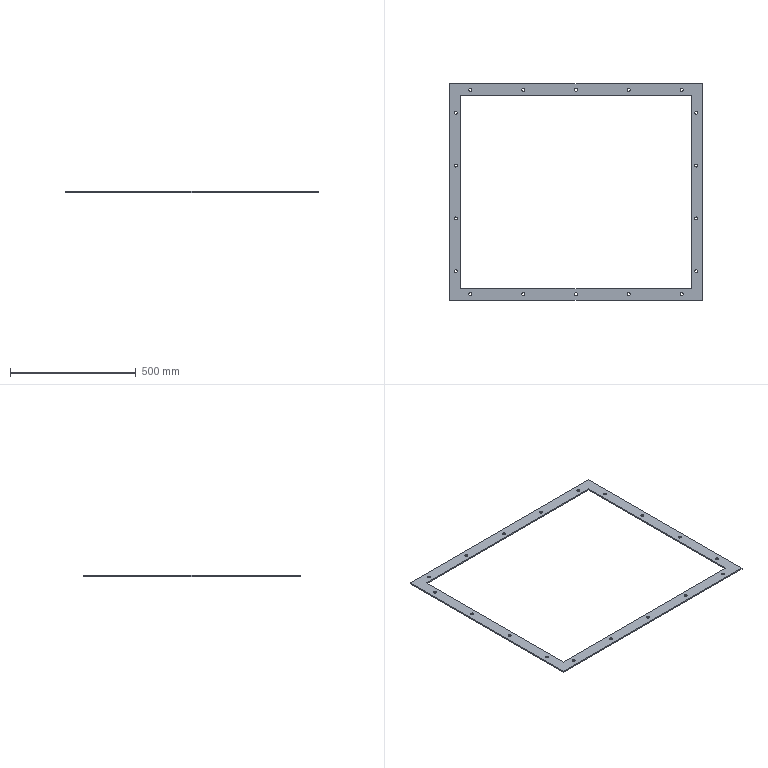Part | STEP file | 750038556 | 1 solid | 46 faces | box 1005 x 861 x 5 mm | volume 789021 mm3 | cylinder 36 | plane 10 | commonest cylinder face diameters 12 x36
STEP:
#1=CARTESIAN_POINT('',(472.,315.,0.));
#2=VERTEX_POINT('',#1);
#3=CARTESIAN_POINT('',(484.,315.,0.));
#4=VERTEX_POINT('',#3);
#5=CARTESIAN_POINT('',(478.,315.,0.));
#6=DIRECTION('',(0.,0.,1.));
#7=DIRECTION('',(1.,0.,0.));
#8=AXIS2_PLACEMENT_3D('',#5,#6,#7);
#9=CIRCLE('',#8,6.);
#10=EDGE_CURVE('',#2,#4,#9,.T.);
#11=ORIENTED_EDGE('',*,*,#10,.F.);
#12=CARTESIAN_POINT('',(472.,315.,5.));
#13=VERTEX_POINT('',#12);
#14=CARTESIAN_POINT('',(472.,315.,-0.5));
#15=DIRECTION('',(0.,0.,1.));
#16=VECTOR('',#15,1000.);
#17=LINE('',#14,#16);
#18=EDGE_CURVE('',#2,#13,#17,.T.);
#19=ORIENTED_EDGE('',*,*,#18,.T.);
#20=CARTESIAN_POINT('',(484.,315.,5.));
#21=VERTEX_POINT('',#20);
#22=CARTESIAN_POINT('',(478.,315.,5.));
#23=DIRECTION('',(0.,0.,-1.));
#24=DIRECTION('',(1.,0.,0.));
#25=AXIS2_PLACEMENT_3D('',#22,#23,#24);
#26=CIRCLE('',#25,6.);
#27=EDGE_CURVE('',#21,#13,#26,.T.);
#28=ORIENTED_EDGE('',*,*,#27,.F.);
#29=CARTESIAN_POINT('',(484.,315.,-0.5));
#30=DIRECTION('',(0.,0.,1.));
#31=VECTOR('',#30,1000.);
#32=LINE('',#29,#31);
#33=EDGE_CURVE('',#4,#21,#32,.T.);
#34=ORIENTED_EDGE('',*,*,#33,.F.);
#35=EDGE_LOOP('',(#11,#19,#28,#34));
#36=FACE_OUTER_BOUND('',#35,.T.);
#37=CARTESIAN_POINT('',(478.,315.,-0.5));
#38=DIRECTION('',(0.,0.,1.));
#39=DIRECTION('',(1.,0.,0.));
#40=AXIS2_PLACEMENT_3D('',#37,#38,#39);
#41=CYLINDRICAL_SURFACE('',#40,6.);
#42=ADVANCED_FACE('',(#36),#41,.F.);
#43=CARTESIAN_POINT('',(-484.,-315.,0.));
#44=VERTEX_POINT('',#43);
#45=CARTESIAN_POINT('',(-472.,-315.,0.));
#46=VERTEX_POINT('',#45);
#47=CARTESIAN_POINT('',(-478.,-315.,0.));
#48=DIRECTION('',(0.,0.,1.));
#49=DIRECTION('',(1.,0.,0.));
#50=AXIS2_PLACEMENT_3D('',#47,#48,#49);
#51=CIRCLE('',#50,6.);
#52=EDGE_CURVE('',#44,#46,#51,.T.);
#53=ORIENTED_EDGE('',*,*,#52,.F.);
#54=CARTESIAN_POINT('',(-484.,-315.,5.));
#55=VERTEX_POINT('',#54);
#56=CARTESIAN_POINT('',(-484.,-315.,-0.5));
#57=DIRECTION('',(0.,0.,1.));
#58=VECTOR('',#57,1000.);
#59=LINE('',#56,#58);
#60=EDGE_CURVE('',#44,#55,#59,.T.);
#61=ORIENTED_EDGE('',*,*,#60,.T.);
#62=CARTESIAN_POINT('',(-472.,-315.,5.));
#63=VERTEX_POINT('',#62);
#64=CARTESIAN_POINT('',(-478.,-315.,5.));
#65=DIRECTION('',(0.,0.,-1.));
#66=DIRECTION('',(1.,0.,0.));
#67=AXIS2_PLACEMENT_3D('',#64,#65,#66);
#68=CIRCLE('',#67,6.);
#69=EDGE_CURVE('',#63,#55,#68,.T.);
#70=ORIENTED_EDGE('',*,*,#69,.F.);
#71=CARTESIAN_POINT('',(-472.,-315.,-0.5));
#72=DIRECTION('',(0.,0.,1.));
#73=VECTOR('',#72,1000.);
#74=LINE('',#71,#73);
#75=EDGE_CURVE('',#46,#63,#74,.T.);
#76=ORIENTED_EDGE('',*,*,#75,.F.);
#77=EDGE_LOOP('',(#53,#61,#70,#76));
#78=FACE_OUTER_BOUND('',#77,.T.);
#79=CARTESIAN_POINT('',(-478.,-315.,-0.5));
#80=DIRECTION('',(0.,0.,1.));
#81=DIRECTION('',(1.,0.,0.));
#82=AXIS2_PLACEMENT_3D('',#79,#80,#81);
#83=CYLINDRICAL_SURFACE('',#82,6.);
#84=ADVANCED_FACE('',(#78),#83,.F.);
#85=CARTESIAN_POINT('',(414.,-406.,0.));
#86=VERTEX_POINT('',#85);
#87=CARTESIAN_POINT('',(426.,-406.,0.));
#88=VERTEX_POINT('',#87);
#89=CARTESIAN_POINT('',(420.,-406.,0.));
#90=DIRECTION('',(0.,0.,1.));
#91=DIRECTION('',(1.,0.,0.));
#92=AXIS2_PLACEMENT_3D('',#89,#90,#91);
#93=CIRCLE('',#92,6.);
#94=EDGE_CURVE('',#86,#88,#93,.T.);
#95=ORIENTED_EDGE('',*,*,#94,.F.);
#96=CARTESIAN_POINT('',(414.,-406.,5.));
#97=VERTEX_POINT('',#96);
#98=CARTESIAN_POINT('',(414.,-406.,-0.5));
#99=DIRECTION('',(0.,0.,1.));
#100=VECTOR('',#99,1000.);
#101=LINE('',#98,#100);
#102=EDGE_CURVE('',#86,#97,#101,.T.);
#103=ORIENTED_EDGE('',*,*,#102,.T.);
#104=CARTESIAN_POINT('',(426.,-406.,5.));
#105=VERTEX_POINT('',#104);
#106=CARTESIAN_POINT('',(420.,-406.,5.));
#107=DIRECTION('',(0.,0.,-1.));
#108=DIRECTION('',(1.,0.,0.));
#109=AXIS2_PLACEMENT_3D('',#106,#107,#108);
#110=CIRCLE('',#109,6.);
#111=EDGE_CURVE('',#105,#97,#110,.T.);
#112=ORIENTED_EDGE('',*,*,#111,.F.);
#113=CARTESIAN_POINT('',(426.,-406.,-0.5));
#114=DIRECTION('',(0.,0.,1.));
#115=VECTOR('',#114,1000.);
#116=LINE('',#113,#115);
#117=EDGE_CURVE('',#88,#105,#116,.T.);
#118=ORIENTED_EDGE('',*,*,#117,.F.);
#119=EDGE_LOOP('',(#95,#103,#112,#118));
#120=FACE_OUTER_BOUND('',#119,.T.);
#121=CARTESIAN_POINT('',(420.,-406.,-0.5));
#122=DIRECTION('',(0.,0.,1.));
#123=DIRECTION('',(1.,0.,0.));
#124=AXIS2_PLACEMENT_3D('',#121,#122,#123);
#125=CYLINDRICAL_SURFACE('',#124,6.);
#126=ADVANCED_FACE('',(#120),#125,.F.);
#127=CARTESIAN_POINT('',(204.,406.,0.));
#128=VERTEX_POINT('',#127);
#129=CARTESIAN_POINT('',(216.,406.,0.));
#130=VERTEX_POINT('',#129);
#131=CARTESIAN_POINT('',(210.,406.,0.));
#132=DIRECTION('',(0.,0.,1.));
#133=DIRECTION('',(1.,0.,0.));
#134=AXIS2_PLACEMENT_3D('',#131,#132,#133);
#135=CIRCLE('',#134,6.);
#136=EDGE_CURVE('',#128,#130,#135,.T.);
#137=ORIENTED_EDGE('',*,*,#136,.F.);
#138=CARTESIAN_POINT('',(204.,406.,5.));
#139=VERTEX_POINT('',#138);
#140=CARTESIAN_POINT('',(204.,406.,-0.5));
#141=DIRECTION('',(0.,0.,1.));
#142=VECTOR('',#141,1000.);
#143=LINE('',#140,#142);
#144=EDGE_CURVE('',#128,#139,#143,.T.);
#145=ORIENTED_EDGE('',*,*,#144,.T.);
#146=CARTESIAN_POINT('',(216.,406.,5.));
#147=VERTEX_POINT('',#146);
#148=CARTESIAN_POINT('',(210.,406.,5.));
#149=DIRECTION('',(0.,0.,-1.));
#150=DIRECTION('',(1.,0.,0.));
#151=AXIS2_PLACEMENT_3D('',#148,#149,#150);
#152=CIRCLE('',#151,6.);
#153=EDGE_CURVE('',#147,#139,#152,.T.);
#154=ORIENTED_EDGE('',*,*,#153,.F.);
#155=CARTESIAN_POINT('',(216.,406.,-0.5));
#156=DIRECTION('',(0.,0.,1.));
#157=VECTOR('',#156,1000.);
#158=LINE('',#155,#157);
#159=EDGE_CURVE('',#130,#147,#158,.T.);
#160=ORIENTED_EDGE('',*,*,#159,.F.);
#161=EDGE_LOOP('',(#137,#145,#154,#160));
#162=FACE_OUTER_BOUND('',#161,.T.);
#163=CARTESIAN_POINT('',(210.,406.,-0.5));
#164=DIRECTION('',(0.,0.,1.));
#165=DIRECTION('',(1.,0.,0.));
#166=AXIS2_PLACEMENT_3D('',#163,#164,#165);
#167=CYLINDRICAL_SURFACE('',#166,6.);
#168=ADVANCED_FACE('',(#162),#167,.F.);
#169=CARTESIAN_POINT('',(204.,-406.,0.));
#170=VERTEX_POINT('',#169);
#171=CARTESIAN_POINT('',(216.,-406.,0.));
#172=VERTEX_POINT('',#171);
#173=CARTESIAN_POINT('',(210.,-406.,0.));
#174=DIRECTION('',(0.,0.,1.));
#175=DIRECTION('',(1.,0.,0.));
#176=AXIS2_PLACEMENT_3D('',#173,#174,#175);
#177=CIRCLE('',#176,6.);
#178=EDGE_CURVE('',#170,#172,#177,.T.);
#179=ORIENTED_EDGE('',*,*,#178,.F.);
#180=CARTESIAN_POINT('',(204.,-406.,5.));
#181=VERTEX_POINT('',#180);
#182=CARTESIAN_POINT('',(204.,-406.,-0.5));
#183=DIRECTION('',(0.,0.,1.));
#184=VECTOR('',#183,1000.);
#185=LINE('',#182,#184);
#186=EDGE_CURVE('',#170,#181,#185,.T.);
#187=ORIENTED_EDGE('',*,*,#186,.T.);
#188=CARTESIAN_POINT('',(216.,-406.,5.));
#189=VERTEX_POINT('',#188);
#190=CARTESIAN_POINT('',(210.,-406.,5.));
#191=DIRECTION('',(0.,0.,-1.));
#192=DIRECTION('',(1.,0.,0.));
#193=AXIS2_PLACEMENT_3D('',#190,#191,#192);
#194=CIRCLE('',#193,6.);
#195=EDGE_CURVE('',#189,#181,#194,.T.);
#196=ORIENTED_EDGE('',*,*,#195,.F.);
#197=CARTESIAN_POINT('',(216.,-406.,-0.5));
#198=DIRECTION('',(0.,0.,1.));
#199=VECTOR('',#198,1000.);
#200=LINE('',#197,#199);
#201=EDGE_CURVE('',#172,#189,#200,.T.);
#202=ORIENTED_EDGE('',*,*,#201,.F.);
#203=EDGE_LOOP('',(#179,#187,#196,#202));
#204=FACE_OUTER_BOUND('',#203,.T.);
#205=CARTESIAN_POINT('',(210.,-406.,-0.5));
#206=DIRECTION('',(0.,0.,1.));
#207=DIRECTION('',(1.,0.,0.));
#208=AXIS2_PLACEMENT_3D('',#205,#206,#207);
#209=CYLINDRICAL_SURFACE('',#208,6.);
#210=ADVANCED_FACE('',(#204),#209,.F.);
#211=CARTESIAN_POINT('',(-6.,406.,0.));
#212=VERTEX_POINT('',#211);
#213=CARTESIAN_POINT('',(6.,406.,0.));
#214=VERTEX_POINT('',#213);
#215=CARTESIAN_POINT('',(0.,406.,0.));
#216=DIRECTION('',(0.,0.,1.));
#217=DIRECTION('',(1.,0.,0.));
#218=AXIS2_PLACEMENT_3D('',#215,#216,#217);
#219=CIRCLE('',#218,6.);
#220=EDGE_CURVE('',#212,#214,#219,.T.);
#221=ORIENTED_EDGE('',*,*,#220,.F.);
#222=CARTESIAN_POINT('',(-6.,406.,5.));
#223=VERTEX_POINT('',#222);
#224=CARTESIAN_POINT('',(-6.,406.,-0.5));
#225=DIRECTION('',(0.,0.,1.));
#226=VECTOR('',#225,1000.);
#227=LINE('',#224,#226);
#228=EDGE_CURVE('',#212,#223,#227,.T.);
#229=ORIENTED_EDGE('',*,*,#228,.T.);
#230=CARTESIAN_POINT('',(6.,406.,5.));
#231=VERTEX_POINT('',#230);
#232=CARTESIAN_POINT('',(0.,406.,5.));
#233=DIRECTION('',(0.,0.,-1.));
#234=DIRECTION('',(1.,0.,0.));
#235=AXIS2_PLACEMENT_3D('',#232,#233,#234);
#236=CIRCLE('',#235,6.);
#237=EDGE_CURVE('',#231,#223,#236,.T.);
#238=ORIENTED_EDGE('',*,*,#237,.F.);
#239=CARTESIAN_POINT('',(6.,406.,-0.5));
#240=DIRECTION('',(0.,0.,1.));
#241=VECTOR('',#240,1000.);
#242=LINE('',#239,#241);
#243=EDGE_CURVE('',#214,#231,#242,.T.);
#244=ORIENTED_EDGE('',*,*,#243,.F.);
#245=EDGE_LOOP('',(#221,#229,#238,#244));
#246=FACE_OUTER_BOUND('',#245,.T.);
#247=CARTESIAN_POINT('',(0.,406.,-0.5));
#248=DIRECTION('',(0.,0.,1.));
#249=DIRECTION('',(1.,0.,0.));
#250=AXIS2_PLACEMENT_3D('',#247,#248,#249);
#251=CYLINDRICAL_SURFACE('',#250,6.);
#252=ADVANCED_FACE('',(#246),#251,.F.);
#253=CARTESIAN_POINT('',(472.,105.,0.));
#254=VERTEX_POINT('',#253);
#255=CARTESIAN_POINT('',(484.,105.,0.));
#256=VERTEX_POINT('',#255);
#257=CARTESIAN_POINT('',(478.,105.,0.));
#258=DIRECTION('',(0.,0.,1.));
#259=DIRECTION('',(1.,0.,0.));
#260=AXIS2_PLACEMENT_3D('',#257,#258,#259);
#261=CIRCLE('',#260,6.);
#262=EDGE_CURVE('',#254,#256,#261,.T.);
#263=ORIENTED_EDGE('',*,*,#262,.F.);
#264=CARTESIAN_POINT('',(472.,105.,5.));
#265=VERTEX_POINT('',#264);
#266=CARTESIAN_POINT('',(472.,105.,-0.5));
#267=DIRECTION('',(0.,0.,1.));
#268=VECTOR('',#267,1000.);
#269=LINE('',#266,#268);
#270=EDGE_CURVE('',#254,#265,#269,.T.);
#271=ORIENTED_EDGE('',*,*,#270,.T.);
#272=CARTESIAN_POINT('',(484.,105.,5.));
#273=VERTEX_POINT('',#272);
#274=CARTESIAN_POINT('',(478.,105.,5.));
#275=DIRECTION('',(0.,0.,-1.));
#276=DIRECTION('',(1.,0.,0.));
#277=AXIS2_PLACEMENT_3D('',#274,#275,#276);
#278=CIRCLE('',#277,6.);
#279=EDGE_CURVE('',#273,#265,#278,.T.);
#280=ORIENTED_EDGE('',*,*,#279,.F.);
#281=CARTESIAN_POINT('',(484.,105.,-0.5));
#282=DIRECTION('',(0.,0.,1.));
#283=VECTOR('',#282,1000.);
#284=LINE('',#281,#283);
#285=EDGE_CURVE('',#256,#273,#284,.T.);
#286=ORIENTED_EDGE('',*,*,#285,.F.);
#287=EDGE_LOOP('',(#263,#271,#280,#286));
#288=FACE_OUTER_BOUND('',#287,.T.);
#289=CARTESIAN_POINT('',(478.,105.,-0.5));
#290=DIRECTION('',(0.,0.,1.));
#291=DIRECTION('',(1.,0.,0.));
#292=AXIS2_PLACEMENT_3D('',#289,#290,#291);
#293=CYLINDRICAL_SURFACE('',#292,6.);
#294=ADVANCED_FACE('',(#288),#293,.F.);
#295=CARTESIAN_POINT('',(472.,-105.,0.));
#296=VERTEX_POINT('',#295);
#297=CARTESIAN_POINT('',(484.,-105.,0.));
#298=VERTEX_POINT('',#297);
#299=CARTESIAN_POINT('',(478.,-105.,0.));
#300=DIRECTION('',(0.,0.,1.));
#301=DIRECTION('',(1.,0.,0.));
#302=AXIS2_PLACEMENT_3D('',#299,#300,#301);
#303=CIRCLE('',#302,6.);
#304=EDGE_CURVE('',#296,#298,#303,.T.);
#305=ORIENTED_EDGE('',*,*,#304,.F.);
#306=CARTESIAN_POINT('',(472.,-105.,5.));
#307=VERTEX_POINT('',#306);
#308=CARTESIAN_POINT('',(472.,-105.,-0.5));
#309=DIRECTION('',(0.,0.,1.));
#310=VECTOR('',#309,1000.);
#311=LINE('',#308,#310);
#312=EDGE_CURVE('',#296,#307,#311,.T.);
#313=ORIENTED_EDGE('',*,*,#312,.T.);
#314=CARTESIAN_POINT('',(484.,-105.,5.));
#315=VERTEX_POINT('',#314);
#316=CARTESIAN_POINT('',(478.,-105.,5.));
#317=DIRECTION('',(0.,0.,-1.));
#318=DIRECTION('',(1.,0.,0.));
#319=AXIS2_PLACEMENT_3D('',#316,#317,#318);
#320=CIRCLE('',#319,6.);
#321=EDGE_CURVE('',#315,#307,#320,.T.);
#322=ORIENTED_EDGE('',*,*,#321,.F.);
#323=CARTESIAN_POINT('',(484.,-105.,-0.5));
#324=DIRECTION('',(0.,0.,1.));
#325=VECTOR('',#324,1000.);
#326=LINE('',#323,#325);
#327=EDGE_CURVE('',#298,#315,#326,.T.);
#328=ORIENTED_EDGE('',*,*,#327,.F.);
#329=EDGE_LOOP('',(#305,#313,#322,#328));
#330=FACE_OUTER_BOUND('',#329,.T.);
#331=CARTESIAN_POINT('',(478.,-105.,-0.5));
#332=DIRECTION('',(0.,0.,1.));
#333=DIRECTION('',(1.,0.,0.));
#334=AXIS2_PLACEMENT_3D('',#331,#332,#333);
#335=CYLINDRICAL_SURFACE('',#334,6.);
#336=ADVANCED_FACE('',(#330),#335,.F.);
#337=CARTESIAN_POINT('',(472.,-315.,0.));
#338=VERTEX_POINT('',#337);
#339=CARTESIAN_POINT('',(484.,-315.,0.));
#340=VERTEX_POINT('',#339);
#341=CARTESIAN_POINT('',(478.,-315.,0.));
#342=DIRECTION('',(0.,0.,1.));
#343=DIRECTION('',(1.,0.,0.));
#344=AXIS2_PLACEMENT_3D('',#341,#342,#343);
#345=CIRCLE('',#344,6.);
#346=EDGE_CURVE('',#338,#340,#345,.T.);
#347=ORIENTED_EDGE('',*,*,#346,.F.);
#348=CARTESIAN_POINT('',(472.,-315.,5.));
#349=VERTEX_POINT('',#348);
#350=CARTESIAN_POINT('',(472.,-315.,-0.5));
#351=DIRECTION('',(0.,0.,1.));
#352=VECTOR('',#351,1000.);
#353=LINE('',#350,#352);
#354=EDGE_CURVE('',#338,#349,#353,.T.);
#355=ORIENTED_EDGE('',*,*,#354,.T.);
#356=CARTESIAN_POINT('',(484.,-315.,5.));
#357=VERTEX_POINT('',#356);
#358=CARTESIAN_POINT('',(478.,-315.,5.));
#359=DIRECTION('',(0.,0.,-1.));
#360=DIRECTION('',(1.,0.,0.));
#361=AXIS2_PLACEMENT_3D('',#358,#359,#360);
#362=CIRCLE('',#361,6.);
#363=EDGE_CURVE('',#357,#349,#362,.T.);
#364=ORIENTED_EDGE('',*,*,#363,.F.);
#365=CARTESIAN_POINT('',(484.,-315.,-0.5));
#366=DIRECTION('',(0.,0.,1.));
#367=VECTOR('',#366,1000.);
#368=LINE('',#365,#367);
#369=EDGE_CURVE('',#340,#357,#368,.T.);
#370=ORIENTED_EDGE('',*,*,#369,.F.);
#371=EDGE_LOOP('',(#347,#355,#364,#370));
#372=FACE_OUTER_BOUND('',#371,.T.);
#373=CARTESIAN_POINT('',(478.,-315.,-0.5));
#374=DIRECTION('',(0.,0.,1.));
#375=DIRECTION('',(1.,0.,0.));
#376=AXIS2_PLACEMENT_3D('',#373,#374,#375);
#377=CYLINDRICAL_SURFACE('',#376,6.);
#378=ADVANCED_FACE('',(#372),#377,.F.);
#379=CARTESIAN_POINT('',(414.,406.,0.));
#380=VERTEX_POINT('',#379);
#381=CARTESIAN_POINT('',(426.,406.,0.));
#382=VERTEX_POINT('',#381);
#383=CARTESIAN_POINT('',(420.,406.,0.));
#384=DIRECTION('',(0.,0.,1.));
#385=DIRECTION('',(1.,0.,0.));
#386=AXIS2_PLACEMENT_3D('',#383,#384,#385);
#387=CIRCLE('',#386,6.);
#388=EDGE_CURVE('',#380,#382,#387,.T.);
#389=ORIENTED_EDGE('',*,*,#388,.F.);
#390=CARTESIAN_POINT('',(414.,406.,5.));
#391=VERTEX_POINT('',#390);
#392=CARTESIAN_POINT('',(414.,406.,-0.5));
#393=DIRECTION('',(0.,0.,1.));
#394=VECTOR('',#393,1000.);
#395=LINE('',#392,#394);
#396=EDGE_CURVE('',#380,#391,#395,.T.);
#397=ORIENTED_EDGE('',*,*,#396,.T.);
#398=CARTESIAN_POINT('',(426.,406.,5.));
#399=VERTEX_POINT('',#398);
#400=CARTESIAN_POINT('',(420.,406.,5.));
#401=DIRECTION('',(0.,0.,-1.));
#402=DIRECTION('',(1.,0.,0.));
#403=AXIS2_PLACEMENT_3D('',#400,#401,#402);
#404=CIRCLE('',#403,6.);
#405=EDGE_CURVE('',#399,#391,#404,.T.);
#406=ORIENTED_EDGE('',*,*,#405,.F.);
#407=CARTESIAN_POINT('',(426.,406.,-0.5));
#408=DIRECTION('',(0.,0.,1.));
#409=VECTOR('',#408,1000.);
#410=LINE('',#407,#409);
#411=EDGE_CURVE('',#382,#399,#410,.T.);
#412=ORIENTED_EDGE('',*,*,#411,.F.);
#413=EDGE_LOOP('',(#389,#397,#406,#412));
#414=FACE_OUTER_BOUND('',#413,.T.);
#415=CARTESIAN_POINT('',(420.,406.,-0.5));
#416=DIRECTION('',(0.,0.,1.));
#417=DIRECTION('',(1.,0.,0.));
#418=AXIS2_PLACEMENT_3D('',#415,#416,#417);
#419=CYLINDRICAL_SURFACE('',#418,6.);
#420=ADVANCED_FACE('',(#414),#419,.F.);
#421=CARTESIAN_POINT('',(-426.,-406.,0.));
#422=VERTEX_POINT('',#421);
#423=CARTESIAN_POINT('',(-414.,-406.,0.));
#424=VERTEX_POINT('',#423);
#425=CARTESIAN_POINT('',(-420.,-406.,0.));
#426=DIRECTION('',(0.,0.,1.));
#427=DIRECTION('',(1.,0.,0.));
#428=AXIS2_PLACEMENT_3D('',#425,#426,#427);
#429=CIRCLE('',#428,6.);
#430=EDGE_CURVE('',#422,#424,#429,.T.);
#431=ORIENTED_EDGE('',*,*,#430,.F.);
#432=CARTESIAN_POINT('',(-426.,-406.,5.));
#433=VERTEX_POINT('',#432);
#434=CARTESIAN_POINT('',(-426.,-406.,-0.5));
#435=DIRECTION('',(0.,0.,1.));
#436=VECTOR('',#435,1000.);
#437=LINE('',#434,#436);
#438=EDGE_CURVE('',#422,#433,#437,.T.);
#439=ORIENTED_EDGE('',*,*,#438,.T.);
#440=CARTESIAN_POINT('',(-414.,-406.,5.));
#441=VERTEX_POINT('',#440);
#442=CARTESIAN_POINT('',(-420.,-406.,5.));
#443=DIRECTION('',(0.,0.,-1.));
#444=DIRECTION('',(1.,0.,0.));
#445=AXIS2_PLACEMENT_3D('',#442,#443,#444);
#446=CIRCLE('',#445,6.);
#447=EDGE_CURVE('',#441,#433,#446,.T.);
#448=ORIENTED_EDGE('',*,*,#447,.F.);
#449=CARTESIAN_POINT('',(-414.,-406.,-0.5));
#450=DIRECTION('',(0.,0.,1.));
#451=VECTOR('',#450,1000.);
#452=LINE('',#449,#451);
#453=EDGE_CURVE('',#424,#441,#452,.T.);
#454=ORIENTED_EDGE('',*,*,#453,.F.);
#455=EDGE_LOOP('',(#431,#439,#448,#454));
#456=FACE_OUTER_BOUND('',#455,.T.);
#457=CARTESIAN_POINT('',(-420.,-406.,-0.5));
#458=DIRECTION('',(0.,0.,1.));
#459=DIRECTION('',(1.,0.,0.));
#460=AXIS2_PLACEMENT_3D('',#457,#458,#459);
#461=CYLINDRICAL_SURFACE('',#460,6.);
#462=ADVANCED_FACE('',(#456),#461,.F.);
#463=CARTESIAN_POINT('',(-484.,315.,0.));
#464=VERTEX_POINT('',#463);
#465=CARTESIAN_POINT('',(-472.,315.,0.));
#466=VERTEX_POINT('',#465);
#467=CARTESIAN_POINT('',(-478.,315.,0.));
#468=DIRECTION('',(0.,0.,1.));
#469=DIRECTION('',(1.,0.,0.));
#470=AXIS2_PLACEMENT_3D('',#467,#468,#469);
#471=CIRCLE('',#470,6.);
#472=EDGE_CURVE('',#464,#466,#471,.T.);
#473=ORIENTED_EDGE('',*,*,#472,.F.);
#474=CARTESIAN_POINT('',(-484.,315.,5.));
#475=VERTEX_POINT('',#474);
#476=CARTESIAN_POINT('',(-484.,315.,-0.5));
#477=DIRECTION('',(0.,0.,1.));
#478=VECTOR('',#477,1000.);
#479=LINE('',#476,#478);
#480=EDGE_CURVE('',#464,#475,#479,.T.);
#481=ORIENTED_EDGE('',*,*,#480,.T.);
#482=CARTESIAN_POINT('',(-472.,315.,5.));
#483=VERTEX_POINT('',#482);
#484=CARTESIAN_POINT('',(-478.,315.,5.));
#485=DIRECTION('',(0.,0.,-1.));
#486=DIRECTION('',(1.,0.,0.));
#487=AXIS2_PLACEMENT_3D('',#484,#485,#486);
#488=CIRCLE('',#487,6.);
#489=EDGE_CURVE('',#483,#475,#488,.T.);
#490=ORIENTED_EDGE('',*,*,#489,.F.);
#491=CARTESIAN_POINT('',(-472.,315.,-0.5));
#492=DIRECTION('',(0.,0.,1.));
#493=VECTOR('',#492,1000.);
#494=LINE('',#491,#493);
#495=EDGE_CURVE('',#466,#483,#494,.T.);
#496=ORIENTED_EDGE('',*,*,#495,.F.);
#497=EDGE_LOOP('',(#473,#481,#490,#496));
#498=FACE_OUTER_BOUND('',#497,.T.);
#499=CARTESIAN_POINT('',(-478.,315.,-0.5));
#500=DIRECTION('',(0.,0.,1.));
#501=DIRECTION('',(1.,0.,0.));
#502=AXIS2_PLACEMENT_3D('',#499,#500,#501);
#503=CYLINDRICAL_SURFACE('',#502,6.);
#504=ADVANCED_FACE('',(#498),#503,.F.);
#505=CARTESIAN_POINT('',(-484.,105.,0.));
#506=VERTEX_POINT('',#505);
#507=CARTESIAN_POINT('',(-472.,105.,0.));
#508=VERTEX_POINT('',#507);
#509=CARTESIAN_POINT('',(-478.,105.,0.));
#510=DIRECTION('',(0.,0.,1.));
#511=DIRECTION('',(1.,0.,0.));
#512=AXIS2_PLACEMENT_3D('',#509,#510,#511);
#513=CIRCLE('',#512,6.);
#514=EDGE_CURVE('',#506,#508,#513,.T.);
#515=ORIENTED_EDGE('',*,*,#514,.F.);
#516=CARTESIAN_POINT('',(-484.,105.,5.));
#517=VERTEX_POINT('',#516);
#518=CARTESIAN_POINT('',(-484.,105.,-0.5));
#519=DIRECTION('',(0.,0.,1.));
#520=VECTOR('',#519,1000.);
#521=LINE('',#518,#520);
#522=EDGE_CURVE('',#506,#517,#521,.T.);
#523=ORIENTED_EDGE('',*,*,#522,.T.);
#524=CARTESIAN_POINT('',(-472.,105.,5.));
#525=VERTEX_POINT('',#524);
#526=CARTESIAN_POINT('',(-478.,105.,5.));
#527=DIRECTION('',(0.,0.,-1.));
#528=DIRECTION('',(1.,0.,0.));
#529=AXIS2_PLACEMENT_3D('',#526,#527,#528);
#530=CIRCLE('',#529,6.);
#531=EDGE_CURVE('',#525,#517,#530,.T.);
#532=ORIENTED_EDGE('',*,*,#531,.F.);
#533=CARTESIAN_POINT('',(-472.,105.,-0.5));
#534=DIRECTION('',(0.,0.,1.));
#535=VECTOR('',#534,1000.);
#536=LINE('',#533,#535);
#537=EDGE_CURVE('',#508,#525,#536,.T.);
#538=ORIENTED_EDGE('',*,*,#537,.F.);
#539=EDGE_LOOP('',(#515,#523,#532,#538));
#540=FACE_OUTER_BOUND('',#539,.T.);
#541=CARTESIAN_POINT('',(-478.,105.,-0.5));
#542=DIRECTION('',(0.,0.,1.));
#543=DIRECTION('',(1.,0.,0.));
#544=AXIS2_PLACEMENT_3D('',#541,#542,#543);
#545=CYLINDRICAL_SURFACE('',#544,6.);
#546=ADVANCED_FACE('',(#540),#545,.F.);
#547=CARTESIAN_POINT('',(-484.,-105.,0.));
#548=VERTEX_POINT('',#547);
#549=CARTESIAN_POINT('',(-472.,-105.,0.));
#550=VERTEX_POINT('',#549);
#551=CARTESIAN_POINT('',(-478.,-105.,0.));
#552=DIRECTION('',(0.,0.,1.));
#553=DIRECTION('',(1.,0.,0.));
#554=AXIS2_PLACEMENT_3D('',#551,#552,#553);
#555=CIRCLE('',#554,6.);
#556=EDGE_CURVE('',#548,#550,#555,.T.);
#557=ORIENTED_EDGE('',*,*,#556,.F.);
#558=CARTESIAN_POINT('',(-484.,-105.,5.));
#559=VERTEX_POINT('',#558);
#560=CARTESIAN_POINT('',(-484.,-105.,-0.5));
#561=DIRECTION('',(0.,0.,1.));
#562=VECTOR('',#561,1000.);
#563=LINE('',#560,#562);
#564=EDGE_CURVE('',#548,#559,#563,.T.);
#565=ORIENTED_EDGE('',*,*,#564,.T.);
#566=CARTESIAN_POINT('',(-472.,-105.,5.));
#567=VERTEX_POINT('',#566);
#568=CARTESIAN_POINT('',(-478.,-105.,5.));
#569=DIRECTION('',(0.,0.,-1.));
#570=DIRECTION('',(1.,0.,0.));
#571=AXIS2_PLACEMENT_3D('',#568,#569,#570);
#572=CIRCLE('',#571,6.);
#573=EDGE_CURVE('',#567,#559,#572,.T.);
#574=ORIENTED_EDGE('',*,*,#573,.F.);
#575=CARTESIAN_POINT('',(-472.,-105.,-0.5));
#576=DIRECTION('',(0.,0.,1.));
#577=VECTOR('',#576,1000.);
#578=LINE('',#575,#577);
#579=EDGE_CURVE('',#550,#567,#578,.T.);
#580=ORIENTED_EDGE('',*,*,#579,.F.);
#581=EDGE_LOOP('',(#557,#565,#574,#580));
#582=FACE_OUTER_BOUND('',#581,.T.);
#583=CARTESIAN_POINT('',(-478.,-105.,-0.5));
#584=DIRECTION('',(0.,0.,1.));
#585=DIRECTION('',(1.,0.,0.));
#586=AXIS2_PLACEMENT_3D('',#583,#584,#585);
#587=CYLINDRICAL_SURFACE('',#586,6.);
#588=ADVANCED_FACE('',(#582),#587,.F.);
#589=CARTESIAN_POINT('',(-6.,-406.,0.));
#590=VERTEX_POINT('',#589);
#591=CARTESIAN_POINT('',(6.,-406.,0.));
#592=VERTEX_POINT('',#591);
#593=CARTESIAN_POINT('',(0.,-406.,0.));
#594=DIRECTION('',(0.,0.,1.));
#595=DIRECTION('',(1.,0.,0.));
#596=AXIS2_PLACEMENT_3D('',#593,#594,#595);
#597=CIRCLE('',#596,6.);
#598=EDGE_CURVE('',#590,#592,#597,.T.);
#599=ORIENTED_EDGE('',*,*,#598,.F.);
#600=CARTESIAN_POINT('',(-6.,-406.,5.));
#601=VERTEX_POINT('',#600);
#602=CARTESIAN_POINT('',(-6.,-406.,-0.5));
#603=DIRECTION('',(0.,0.,1.));
#604=VECTOR('',#603,1000.);
#605=LINE('',#602,#604);
#606=EDGE_CURVE('',#590,#601,#605,.T.);
#607=ORIENTED_EDGE('',*,*,#606,.T.);
#608=CARTESIAN_POINT('',(6.,-406.,5.));
#609=VERTEX_POINT('',#608);
#610=CARTESIAN_POINT('',(0.,-406.,5.));
#611=DIRECTION('',(0.,0.,-1.));
#612=DIRECTION('',(1.,0.,0.));
#613=AXIS2_PLACEMENT_3D('',#610,#611,#612);
#614=CIRCLE('',#613,6.);
#615=EDGE_CURVE('',#609,#601,#614,.T.);
#616=ORIENTED_EDGE('',*,*,#615,.F.);
#617=CARTESIAN_POINT('',(6.,-406.,-0.5));
#618=DIRECTION('',(0.,0.,1.));
#619=VECTOR('',#618,1000.);
#620=LINE('',#617,#619);
#621=EDGE_CURVE('',#592,#609,#620,.T.);
#622=ORIENTED_EDGE('',*,*,#621,.F.);
#623=EDGE_LOOP('',(#599,#607,#616,#622));
#624=FACE_OUTER_BOUND('',#623,.T.);
#625=CARTESIAN_POINT('',(0.,-406.,-0.5));
#626=DIRECTION('',(0.,0.,1.));
#627=DIRECTION('',(1.,0.,0.));
#628=AXIS2_PLACEMENT_3D('',#625,#626,#627);
#629=CYLINDRICAL_SURFACE('',#628,6.);
#630=ADVANCED_FACE('',(#624),#629,.F.);
#631=CARTESIAN_POINT('',(-216.,406.,0.));
#632=VERTEX_POINT('',#631);
#633=CARTESIAN_POINT('',(-204.,406.,0.));
#634=VERTEX_POINT('',#633);
#635=CARTESIAN_POINT('',(-210.,406.,0.));
#636=DIRECTION('',(0.,0.,1.));
#637=DIRECTION('',(1.,0.,0.));
#638=AXIS2_PLACEMENT_3D('',#635,#636,#637);
#639=CIRCLE('',#638,6.);
#640=EDGE_CURVE('',#632,#634,#639,.T.);
#641=ORIENTED_EDGE('',*,*,#640,.F.);
#642=CARTESIAN_POINT('',(-216.,406.,5.));
#643=VERTEX_POINT('',#642);
#644=CARTESIAN_POINT('',(-216.,406.,-0.5));
#645=DIRECTION('',(0.,0.,1.));
#646=VECTOR('',#645,1000.);
#647=LINE('',#644,#646);
#648=EDGE_CURVE('',#632,#643,#647,.T.);
#649=ORIENTED_EDGE('',*,*,#648,.T.);
#650=CARTESIAN_POINT('',(-204.,406.,5.));
#651=VERTEX_POINT('',#650);
#652=CARTESIAN_POINT('',(-210.,406.,5.));
#653=DIRECTION('',(0.,0.,-1.));
#654=DIRECTION('',(1.,0.,0.));
#655=AXIS2_PLACEMENT_3D('',#652,#653,#654);
#656=CIRCLE('',#655,6.);
#657=EDGE_CURVE('',#651,#643,#656,.T.);
#658=ORIENTED_EDGE('',*,*,#657,.F.);
#659=CARTESIAN_POINT('',(-204.,406.,-0.5));
#660=DIRECTION('',(0.,0.,1.));
#661=VECTOR('',#660,1000.);
#662=LINE('',#659,#661);
#663=EDGE_CURVE('',#634,#651,#662,.T.);
#664=ORIENTED_EDGE('',*,*,#663,.F.);
#665=EDGE_LOOP('',(#641,#649,#658,#664));
#666=FACE_OUTER_BOUND('',#665,.T.);
#667=CARTESIAN_POINT('',(-210.,406.,-0.5));
#668=DIRECTION('',(0.,0.,1.));
#669=DIRECTION('',(1.,0.,0.));
#670=AXIS2_PLACEMENT_3D('',#667,#668,#669);
#671=CYLINDRICAL_SURFACE('',#670,6.);
#672=ADVANCED_FACE('',(#666),#671,.F.);
#673=CARTESIAN_POINT('',(-216.,-406.,0.));
#674=VERTEX_POINT('',#673);
#675=CARTESIAN_POINT('',(-204.,-406.,0.));
#676=VERTEX_POINT('',#675);
#677=CARTESIAN_POINT('',(-210.,-406.,0.));
#678=DIRECTION('',(0.,0.,1.));
#679=DIRECTION('',(1.,0.,0.));
#680=AXIS2_PLACEMENT_3D('',#677,#678,#679);
#681=CIRCLE('',#680,6.);
#682=EDGE_CURVE('',#674,#676,#681,.T.);
#683=ORIENTED_EDGE('',*,*,#682,.F.);
#684=CARTESIAN_POINT('',(-216.,-406.,5.));
#685=VERTEX_POINT('',#684);
#686=CARTESIAN_POINT('',(-216.,-406.,-0.5));
#687=DIRECTION('',(0.,0.,1.));
#688=VECTOR('',#687,1000.);
#689=LINE('',#686,#688);
#690=EDGE_CURVE('',#674,#685,#689,.T.);
#691=ORIENTED_EDGE('',*,*,#690,.T.);
#692=CARTESIAN_POINT('',(-204.,-406.,5.));
#693=VERTEX_POINT('',#692);
#694=CARTESIAN_POINT('',(-210.,-406.,5.));
#695=DIRECTION('',(0.,0.,-1.));
#696=DIRECTION('',(1.,0.,0.));
#697=AXIS2_PLACEMENT_3D('',#694,#695,#696);
#698=CIRCLE('',#697,6.);
#699=EDGE_CURVE('',#693,#685,#698,.T.);
#700=ORIENTED_EDGE('',*,*,#699,.F.);
#701=CARTESIAN_POINT('',(-204.,-406.,-0.5));
#702=DIRECTION('',(0.,0.,1.));
#703=VECTOR('',#702,1000.);
#704=LINE('',#701,#703);
#705=EDGE_CURVE('',#676,#693,#704,.T.);
#706=ORIENTED_EDGE('',*,*,#705,.F.);
#707=EDGE_LOOP('',(#683,#691,#700,#706));
#708=FACE_OUTER_BOUND('',#707,.T.);
#709=CARTESIAN_POINT('',(-210.,-406.,-0.5));
#710=DIRECTION('',(0.,0.,1.));
#711=DIRECTION('',(1.,0.,0.));
#712=AXIS2_PLACEMENT_3D('',#709,#710,#711);
#713=CYLINDRICAL_SURFACE('',#712,6.);
#714=ADVANCED_FACE('',(#708),#713,.F.);
#715=CARTESIAN_POINT('',(-426.,406.,0.));
#716=VERTEX_POINT('',#715);
#717=CARTESIAN_POINT('',(-414.,406.,0.));
#718=VERTEX_POINT('',#717);
#719=CARTESIAN_POINT('',(-420.,406.,0.));
#720=DIRECTION('',(0.,0.,1.));
#721=DIRECTION('',(1.,0.,0.));
#722=AXIS2_PLACEMENT_3D('',#719,#720,#721);
#723=CIRCLE('',#722,6.);
#724=EDGE_CURVE('',#716,#718,#723,.T.);
#725=ORIENTED_EDGE('',*,*,#724,.F.);
#726=CARTESIAN_POINT('',(-426.,406.,5.));
#727=VERTEX_POINT('',#726);
#728=CARTESIAN_POINT('',(-426.,406.,-0.5));
#729=DIRECTION('',(0.,0.,1.));
#730=VECTOR('',#729,1000.);
#731=LINE('',#728,#730);
#732=EDGE_CURVE('',#716,#727,#731,.T.);
#733=ORIENTED_EDGE('',*,*,#732,.T.);
#734=CARTESIAN_POINT('',(-414.,406.,5.));
#735=VERTEX_POINT('',#734);
#736=CARTESIAN_POINT('',(-420.,406.,5.));
#737=DIRECTION('',(0.,0.,-1.));
#738=DIRECTION('',(1.,0.,0.));
#739=AXIS2_PLACEMENT_3D('',#736,#737,#738);
#740=CIRCLE('',#739,6.);
#741=EDGE_CURVE('',#735,#727,#740,.T.);
#742=ORIENTED_EDGE('',*,*,#741,.F.);
#743=CARTESIAN_POINT('',(-414.,406.,-0.5));
#744=DIRECTION('',(0.,0.,1.));
#745=VECTOR('',#744,1000.);
#746=LINE('',#743,#745);
#747=EDGE_CURVE('',#718,#735,#746,.T.);
#748=ORIENTED_EDGE('',*,*,#747,.F.);
#749=EDGE_LOOP('',(#725,#733,#742,#748));
#750=FACE_OUTER_BOUND('',#749,.T.);
#751=CARTESIAN_POINT('',(-420.,406.,-0.5));
#752=DIRECTION('',(0.,0.,1.));
#753=DIRECTION('',(1.,0.,0.));
#754=AXIS2_PLACEMENT_3D('',#751,#752,#753);
#755=CYLINDRICAL_SURFACE('',#754,6.);
#756=ADVANCED_FACE('',(#750),#755,.F.);
#757=CARTESIAN_POINT('',(457.5,385.5,5.));
#758=VERTEX_POINT('',#757);
#759=CARTESIAN_POINT('',(457.5,-385.5,5.));
#760=VERTEX_POINT('',#759);
#761=CARTESIAN_POINT('',(457.5,0.,5.));
#762=DIRECTION('',(0.,-1.,0.));
#763=VECTOR('',#762,1000.);
#764=LINE('',#761,#763);
#765=EDGE_CURVE('',#758,#760,#764,.T.);
#766=ORIENTED_EDGE('',*,*,#765,.T.);
#767=CARTESIAN_POINT('',(-457.5,-385.5,5.));
#768=VERTEX_POINT('',#767);
#769=CARTESIAN_POINT('',(0.,-385.5,5.));
#770=DIRECTION('',(-1.,0.,0.));
#771=VECTOR('',#770,1000.);
#772=LINE('',#769,#771);
#773=EDGE_CURVE('',#760,#768,#772,.T.);
#774=ORIENTED_EDGE('',*,*,#773,.T.);
#775=CARTESIAN_POINT('',(-457.5,385.5,5.));
#776=VERTEX_POINT('',#775);
#777=CARTESIAN_POINT('',(-457.5,0.,5.));
#778=DIRECTION('',(0.,1.,0.));
#779=VECTOR('',#778,1000.);
#780=LINE('',#777,#779);
#781=EDGE_CURVE('',#768,#776,#780,.T.);
#782=ORIENTED_EDGE('',*,*,#781,.T.);
#783=CARTESIAN_POINT('',(0.,385.5,5.));
#784=DIRECTION('',(1.,0.,0.));
#785=VECTOR('',#784,1000.);
#786=LINE('',#783,#785);
#787=EDGE_CURVE('',#776,#758,#786,.T.);
#788=ORIENTED_EDGE('',*,*,#787,.T.);
#789=EDGE_LOOP('',(#766,#774,#782,#788));
#790=FACE_BOUND('',#789,.T.);
#791=CARTESIAN_POINT('',(502.5,-430.5,5.));
#792=VERTEX_POINT('',#791);
#793=CARTESIAN_POINT('',(502.5,430.5,5.));
#794=VERTEX_POINT('',#793);
#795=CARTESIAN_POINT('',(502.5,0.,5.));
#796=DIRECTION('',(0.,1.,0.));
#797=VECTOR('',#796,1000.);
#798=LINE('',#795,#797);
#799=EDGE_CURVE('',#792,#794,#798,.T.);
#800=ORIENTED_EDGE('',*,*,#799,.T.);
#801=CARTESIAN_POINT('',(-502.5,430.5,5.));
#802=VERTEX_POINT('',#801);
#803=CARTESIAN_POINT('',(0.,430.5,5.));
#804=DIRECTION('',(-1.,0.,0.));
#805=VECTOR('',#804,1000.);
#806=LINE('',#803,#805);
#807=EDGE_CURVE('',#794,#802,#806,.T.);
#808=ORIENTED_EDGE('',*,*,#807,.T.);
#809=CARTESIAN_POINT('',(-502.5,-430.5,5.));
#810=VERTEX_POINT('',#809);
#811=CARTESIAN_POINT('',(-502.5,0.,5.));
#812=DIRECTION('',(0.,-1.,0.));
#813=VECTOR('',#812,1000.);
#814=LINE('',#811,#813);
#815=EDGE_CURVE('',#802,#810,#814,.T.);
#816=ORIENTED_EDGE('',*,*,#815,.T.);
#817=CARTESIAN_POINT('',(0.,-430.5,5.));
#818=DIRECTION('',(1.,0.,0.));
#819=VECTOR('',#818,1000.);
#820=LINE('',#817,#819);
#821=EDGE_CURVE('',#810,#792,#820,.T.);
#822=ORIENTED_EDGE('',*,*,#821,.T.);
#823=EDGE_LOOP('',(#800,#808,#816,#822));
#824=FACE_OUTER_BOUND('',#823,.T.);
#825=ORIENTED_EDGE('',*,*,#27,.T.);
#826=CARTESIAN_POINT('',(478.,315.,5.));
#827=DIRECTION('',(0.,0.,-1.));
#828=DIRECTION('',(1.,0.,0.));
#829=AXIS2_PLACEMENT_3D('',#826,#827,#828);
#830=CIRCLE('',#829,6.);
#831=EDGE_CURVE('',#13,#21,#830,.T.);
#832=ORIENTED_EDGE('',*,*,#831,.T.);
#833=EDGE_LOOP('',(#825,#832));
#834=FACE_BOUND('',#833,.T.);
#835=ORIENTED_EDGE('',*,*,#69,.T.);
#836=CARTESIAN_POINT('',(-478.,-315.,5.));
#837=DIRECTION('',(0.,0.,-1.));
#838=DIRECTION('',(1.,0.,0.));
#839=AXIS2_PLACEMENT_3D('',#836,#837,#838);
#840=CIRCLE('',#839,6.);
#841=EDGE_CURVE('',#55,#63,#840,.T.);
#842=ORIENTED_EDGE('',*,*,#841,.T.);
#843=EDGE_LOOP('',(#835,#842));
#844=FACE_BOUND('',#843,.T.);
#845=ORIENTED_EDGE('',*,*,#111,.T.);
#846=CARTESIAN_POINT('',(420.,-406.,5.));
#847=DIRECTION('',(0.,0.,-1.));
#848=DIRECTION('',(1.,0.,0.));
#849=AXIS2_PLACEMENT_3D('',#846,#847,#848);
#850=CIRCLE('',#849,6.);
#851=EDGE_CURVE('',#97,#105,#850,.T.);
#852=ORIENTED_EDGE('',*,*,#851,.T.);
#853=EDGE_LOOP('',(#845,#852));
#854=FACE_BOUND('',#853,.T.);
#855=ORIENTED_EDGE('',*,*,#153,.T.);
#856=CARTESIAN_POINT('',(210.,406.,5.));
#857=DIRECTION('',(0.,0.,-1.));
#858=DIRECTION('',(1.,0.,0.));
#859=AXIS2_PLACEMENT_3D('',#856,#857,#858);
#860=CIRCLE('',#859,6.);
#861=EDGE_CURVE('',#139,#147,#860,.T.);
#862=ORIENTED_EDGE('',*,*,#861,.T.);
#863=EDGE_LOOP('',(#855,#862));
#864=FACE_BOUND('',#863,.T.);
#865=ORIENTED_EDGE('',*,*,#195,.T.);
#866=CARTESIAN_POINT('',(210.,-406.,5.));
#867=DIRECTION('',(0.,0.,-1.));
#868=DIRECTION('',(1.,0.,0.));
#869=AXIS2_PLACEMENT_3D('',#866,#867,#868);
#870=CIRCLE('',#869,6.);
#871=EDGE_CURVE('',#181,#189,#870,.T.);
#872=ORIENTED_EDGE('',*,*,#871,.T.);
#873=EDGE_LOOP('',(#865,#872));
#874=FACE_BOUND('',#873,.T.);
#875=ORIENTED_EDGE('',*,*,#237,.T.);
#876=CARTESIAN_POINT('',(0.,406.,5.));
#877=DIRECTION('',(0.,0.,-1.));
#878=DIRECTION('',(1.,0.,0.));
#879=AXIS2_PLACEMENT_3D('',#876,#877,#878);
#880=CIRCLE('',#879,6.);
#881=EDGE_CURVE('',#223,#231,#880,.T.);
#882=ORIENTED_EDGE('',*,*,#881,.T.);
#883=EDGE_LOOP('',(#875,#882));
#884=FACE_BOUND('',#883,.T.);
#885=ORIENTED_EDGE('',*,*,#279,.T.);
#886=CARTESIAN_POINT('',(478.,105.,5.));
#887=DIRECTION('',(0.,0.,-1.));
#888=DIRECTION('',(1.,0.,0.));
#889=AXIS2_PLACEMENT_3D('',#886,#887,#888);
#890=CIRCLE('',#889,6.);
#891=EDGE_CURVE('',#265,#273,#890,.T.);
#892=ORIENTED_EDGE('',*,*,#891,.T.);
#893=EDGE_LOOP('',(#885,#892));
#894=FACE_BOUND('',#893,.T.);
#895=ORIENTED_EDGE('',*,*,#321,.T.);
#896=CARTESIAN_POINT('',(478.,-105.,5.));
#897=DIRECTION('',(0.,0.,-1.));
#898=DIRECTION('',(1.,0.,0.));
#899=AXIS2_PLACEMENT_3D('',#896,#897,#898);
#900=CIRCLE('',#899,6.);
#901=EDGE_CURVE('',#307,#315,#900,.T.);
#902=ORIENTED_EDGE('',*,*,#901,.T.);
#903=EDGE_LOOP('',(#895,#902));
#904=FACE_BOUND('',#903,.T.);
#905=ORIENTED_EDGE('',*,*,#363,.T.);
#906=CARTESIAN_POINT('',(478.,-315.,5.));
#907=DIRECTION('',(0.,0.,-1.));
#908=DIRECTION('',(1.,0.,0.));
#909=AXIS2_PLACEMENT_3D('',#906,#907,#908);
#910=CIRCLE('',#909,6.);
#911=EDGE_CURVE('',#349,#357,#910,.T.);
#912=ORIENTED_EDGE('',*,*,#911,.T.);
#913=EDGE_LOOP('',(#905,#912));
#914=FACE_BOUND('',#913,.T.);
#915=ORIENTED_EDGE('',*,*,#405,.T.);
#916=CARTESIAN_POINT('',(420.,406.,5.));
#917=DIRECTION('',(0.,0.,-1.));
#918=DIRECTION('',(1.,0.,0.));
#919=AXIS2_PLACEMENT_3D('',#916,#917,#918);
#920=CIRCLE('',#919,6.);
#921=EDGE_CURVE('',#391,#399,#920,.T.);
#922=ORIENTED_EDGE('',*,*,#921,.T.);
#923=EDGE_LOOP('',(#915,#922));
#924=FACE_BOUND('',#923,.T.);
#925=ORIENTED_EDGE('',*,*,#447,.T.);
#926=CARTESIAN_POINT('',(-420.,-406.,5.));
#927=DIRECTION('',(0.,0.,-1.));
#928=DIRECTION('',(1.,0.,0.));
#929=AXIS2_PLACEMENT_3D('',#926,#927,#928);
#930=CIRCLE('',#929,6.);
#931=EDGE_CURVE('',#433,#441,#930,.T.);
#932=ORIENTED_EDGE('',*,*,#931,.T.);
#933=EDGE_LOOP('',(#925,#932));
#934=FACE_BOUND('',#933,.T.);
#935=ORIENTED_EDGE('',*,*,#489,.T.);
#936=CARTESIAN_POINT('',(-478.,315.,5.));
#937=DIRECTION('',(0.,0.,-1.));
#938=DIRECTION('',(1.,0.,0.));
#939=AXIS2_PLACEMENT_3D('',#936,#937,#938);
#940=CIRCLE('',#939,6.);
#941=EDGE_CURVE('',#475,#483,#940,.T.);
#942=ORIENTED_EDGE('',*,*,#941,.T.);
#943=EDGE_LOOP('',(#935,#942));
#944=FACE_BOUND('',#943,.T.);
#945=ORIENTED_EDGE('',*,*,#531,.T.);
#946=CARTESIAN_POINT('',(-478.,105.,5.));
#947=DIRECTION('',(0.,0.,-1.));
#948=DIRECTION('',(1.,0.,0.));
#949=AXIS2_PLACEMENT_3D('',#946,#947,#948);
#950=CIRCLE('',#949,6.);
#951=EDGE_CURVE('',#517,#525,#950,.T.);
#952=ORIENTED_EDGE('',*,*,#951,.T.);
#953=EDGE_LOOP('',(#945,#952));
#954=FACE_BOUND('',#953,.T.);
#955=ORIENTED_EDGE('',*,*,#573,.T.);
#956=CARTESIAN_POINT('',(-478.,-105.,5.));
#957=DIRECTION('',(0.,0.,-1.));
#958=DIRECTION('',(1.,0.,0.));
#959=AXIS2_PLACEMENT_3D('',#956,#957,#958);
#960=CIRCLE('',#959,6.);
#961=EDGE_CURVE('',#559,#567,#960,.T.);
#962=ORIENTED_EDGE('',*,*,#961,.T.);
#963=EDGE_LOOP('',(#955,#962));
#964=FACE_BOUND('',#963,.T.);
#965=ORIENTED_EDGE('',*,*,#615,.T.);
#966=CARTESIAN_POINT('',(0.,-406.,5.));
#967=DIRECTION('',(0.,0.,-1.));
#968=DIRECTION('',(1.,0.,0.));
#969=AXIS2_PLACEMENT_3D('',#966,#967,#968);
#970=CIRCLE('',#969,6.);
#971=EDGE_CURVE('',#601,#609,#970,.T.);
#972=ORIENTED_EDGE('',*,*,#971,.T.);
#973=EDGE_LOOP('',(#965,#972));
#974=FACE_BOUND('',#973,.T.);
#975=ORIENTED_EDGE('',*,*,#657,.T.);
#976=CARTESIAN_POINT('',(-210.,406.,5.));
#977=DIRECTION('',(0.,0.,-1.));
#978=DIRECTION('',(1.,0.,0.));
#979=AXIS2_PLACEMENT_3D('',#976,#977,#978);
#980=CIRCLE('',#979,6.);
#981=EDGE_CURVE('',#643,#651,#980,.T.);
#982=ORIENTED_EDGE('',*,*,#981,.T.);
#983=EDGE_LOOP('',(#975,#982));
#984=FACE_BOUND('',#983,.T.);
#985=ORIENTED_EDGE('',*,*,#699,.T.);
#986=CARTESIAN_POINT('',(-210.,-406.,5.));
#987=DIRECTION('',(0.,0.,-1.));
#988=DIRECTION('',(1.,0.,0.));
#989=AXIS2_PLACEMENT_3D('',#986,#987,#988);
#990=CIRCLE('',#989,6.);
#991=EDGE_CURVE('',#685,#693,#990,.T.);
#992=ORIENTED_EDGE('',*,*,#991,.T.);
#993=EDGE_LOOP('',(#985,#992));
#994=FACE_BOUND('',#993,.T.);
#995=ORIENTED_EDGE('',*,*,#741,.T.);
#996=CARTESIAN_POINT('',(-420.,406.,5.));
#997=DIRECTION('',(0.,0.,-1.));
#998=DIRECTION('',(1.,0.,0.));
#999=AXIS2_PLACEMENT_3D('',#996,#997,#998);
#1000=CIRCLE('',#999,6.);
#1001=EDGE_CURVE('',#727,#735,#1000,.T.);
#1002=ORIENTED_EDGE('',*,*,#1001,.T.);
#1003=EDGE_LOOP('',(#995,#1002));
#1004=FACE_BOUND('',#1003,.T.);
#1005=CARTESIAN_POINT('',(0.,0.,5.));
#1006=DIRECTION('',(0.,0.,1.));
#1007=DIRECTION('',(1.,0.,0.));
#1008=AXIS2_PLACEMENT_3D('',#1005,#1006,#1007);
#1009=PLANE('',#1008);
#1010=ADVANCED_FACE('',(#790,#824,#834,#844,#854,#864,#874,#884,#894,#904,#914,#924,#934,#944,#954,#964,#974,#984,#994,#1004),#1009,.T.);
#1011=CARTESIAN_POINT('',(-457.5,-385.5,0.));
#1012=VERTEX_POINT('',#1011);
#1013=CARTESIAN_POINT('',(-457.5,-385.5,5.));
#1014=DIRECTION('',(0.,0.,-1.));
#1015=VECTOR('',#1014,1000.);
#1016=LINE('',#1013,#1015);
#1017=EDGE_CURVE('',#768,#1012,#1016,.T.);
#1018=ORIENTED_EDGE('',*,*,#1017,.F.);
#1019=ORIENTED_EDGE('',*,*,#773,.F.);
#1020=CARTESIAN_POINT('',(457.5,-385.5,0.));
#1021=VERTEX_POINT('',#1020);
#1022=CARTESIAN_POINT('',(457.5,-385.5,5.));
#1023=DIRECTION('',(0.,0.,1.));
#1024=VECTOR('',#1023,1000.);
#1025=LINE('',#1022,#1024);
#1026=EDGE_CURVE('',#1021,#760,#1025,.T.);
#1027=ORIENTED_EDGE('',*,*,#1026,.F.);
#1028=CARTESIAN_POINT('',(457.5,-385.5,0.));
#1029=DIRECTION('',(1.,0.,0.));
#1030=VECTOR('',#1029,1000.);
#1031=LINE('',#1028,#1030);
#1032=EDGE_CURVE('',#1012,#1021,#1031,.T.);
#1033=ORIENTED_EDGE('',*,*,#1032,.F.);
#1034=EDGE_LOOP('',(#1018,#1019,#1027,#1033));
#1035=FACE_OUTER_BOUND('',#1034,.T.);
#1036=CARTESIAN_POINT('',(457.5,-385.5,5.));
#1037=DIRECTION('',(0.,-1.,0.));
#1038=DIRECTION('',(0.,0.,-1.));
#1039=AXIS2_PLACEMENT_3D('',#1036,#1037,#1038);
#1040=PLANE('',#1039);
#1041=ADVANCED_FACE('',(#1035),#1040,.F.);
#1042=ORIENTED_EDGE('',*,*,#1026,.T.);
#1043=ORIENTED_EDGE('',*,*,#765,.F.);
#1044=CARTESIAN_POINT('',(457.5,385.5,0.));
#1045=VERTEX_POINT('',#1044);
#1046=CARTESIAN_POINT('',(457.5,385.5,5.));
#1047=DIRECTION('',(0.,0.,1.));
#1048=VECTOR('',#1047,1000.);
#1049=LINE('',#1046,#1048);
#1050=EDGE_CURVE('',#1045,#758,#1049,.T.);
#1051=ORIENTED_EDGE('',*,*,#1050,.F.);
#1052=CARTESIAN_POINT('',(457.5,385.5,0.));
#1053=DIRECTION('',(0.,1.,0.));
#1054=VECTOR('',#1053,1000.);
#1055=LINE('',#1052,#1054);
#1056=EDGE_CURVE('',#1021,#1045,#1055,.T.);
#1057=ORIENTED_EDGE('',*,*,#1056,.F.);
#1058=EDGE_LOOP('',(#1042,#1043,#1051,#1057));
#1059=FACE_OUTER_BOUND('',#1058,.T.);
#1060=CARTESIAN_POINT('',(457.5,385.5,5.));
#1061=DIRECTION('',(1.,0.,0.));
#1062=DIRECTION('',(0.,1.,0.));
#1063=AXIS2_PLACEMENT_3D('',#1060,#1061,#1062);
#1064=PLANE('',#1063);
#1065=ADVANCED_FACE('',(#1059),#1064,.F.);
#1066=ORIENTED_EDGE('',*,*,#1050,.T.);
#1067=ORIENTED_EDGE('',*,*,#787,.F.);
#1068=CARTESIAN_POINT('',(-457.5,385.5,0.));
#1069=VERTEX_POINT('',#1068);
#1070=CARTESIAN_POINT('',(-457.5,385.5,5.));
#1071=DIRECTION('',(0.,0.,1.));
#1072=VECTOR('',#1071,1000.);
#1073=LINE('',#1070,#1072);
#1074=EDGE_CURVE('',#1069,#776,#1073,.T.);
#1075=ORIENTED_EDGE('',*,*,#1074,.F.);
#1076=CARTESIAN_POINT('',(-457.5,385.5,0.));
#1077=DIRECTION('',(-1.,0.,0.));
#1078=VECTOR('',#1077,1000.);
#1079=LINE('',#1076,#1078);
#1080=EDGE_CURVE('',#1045,#1069,#1079,.T.);
#1081=ORIENTED_EDGE('',*,*,#1080,.F.);
#1082=EDGE_LOOP('',(#1066,#1067,#1075,#1081));
#1083=FACE_OUTER_BOUND('',#1082,.T.);
#1084=CARTESIAN_POINT('',(-457.5,385.5,5.));
#1085=DIRECTION('',(0.,1.,0.));
#1086=DIRECTION('',(0.,0.,1.));
#1087=AXIS2_PLACEMENT_3D('',#1084,#1085,#1086);
#1088=PLANE('',#1087);
#1089=ADVANCED_FACE('',(#1083),#1088,.F.);
#1090=ORIENTED_EDGE('',*,*,#1074,.T.);
#1091=ORIENTED_EDGE('',*,*,#781,.F.);
#1092=ORIENTED_EDGE('',*,*,#1017,.T.);
#1093=CARTESIAN_POINT('',(-457.5,-385.5,0.));
#1094=DIRECTION('',(0.,-1.,0.));
#1095=VECTOR('',#1094,1000.);
#1096=LINE('',#1093,#1095);
#1097=EDGE_CURVE('',#1069,#1012,#1096,.T.);
#1098=ORIENTED_EDGE('',*,*,#1097,.F.);
#1099=EDGE_LOOP('',(#1090,#1091,#1092,#1098));
#1100=FACE_OUTER_BOUND('',#1099,.T.);
#1101=CARTESIAN_POINT('',(-457.5,-385.5,5.));
#1102=DIRECTION('',(-1.,0.,0.));
#1103=DIRECTION('',(0.,-1.,0.));
#1104=AXIS2_PLACEMENT_3D('',#1101,#1102,#1103);
#1105=PLANE('',#1104);
#1106=ADVANCED_FACE('',(#1100),#1105,.F.);
#1107=CARTESIAN_POINT('',(-502.5,430.5,0.));
#1108=VERTEX_POINT('',#1107);
#1109=CARTESIAN_POINT('',(-502.5,430.5,5.));
#1110=DIRECTION('',(0.,0.,-1.));
#1111=VECTOR('',#1110,1000.);
#1112=LINE('',#1109,#1111);
#1113=EDGE_CURVE('',#802,#1108,#1112,.T.);
#1114=ORIENTED_EDGE('',*,*,#1113,.F.);
#1115=ORIENTED_EDGE('',*,*,#807,.F.);
#1116=CARTESIAN_POINT('',(502.5,430.5,0.));
#1117=VERTEX_POINT('',#1116);
#1118=CARTESIAN_POINT('',(502.5,430.5,5.));
#1119=DIRECTION('',(0.,0.,1.));
#1120=VECTOR('',#1119,1000.);
#1121=LINE('',#1118,#1120);
#1122=EDGE_CURVE('',#1117,#794,#1121,.T.);
#1123=ORIENTED_EDGE('',*,*,#1122,.F.);
#1124=CARTESIAN_POINT('',(502.5,430.5,0.));
#1125=DIRECTION('',(1.,0.,0.));
#1126=VECTOR('',#1125,1000.);
#1127=LINE('',#1124,#1126);
#1128=EDGE_CURVE('',#1108,#1117,#1127,.T.);
#1129=ORIENTED_EDGE('',*,*,#1128,.F.);
#1130=EDGE_LOOP('',(#1114,#1115,#1123,#1129));
#1131=FACE_OUTER_BOUND('',#1130,.T.);
#1132=CARTESIAN_POINT('',(502.5,430.5,5.));
#1133=DIRECTION('',(0.,-1.,0.));
#1134=DIRECTION('',(0.,0.,-1.));
#1135=AXIS2_PLACEMENT_3D('',#1132,#1133,#1134);
#1136=PLANE('',#1135);
#1137=ADVANCED_FACE('',(#1131),#1136,.F.);
#1138=ORIENTED_EDGE('',*,*,#1122,.T.);
#1139=ORIENTED_EDGE('',*,*,#799,.F.);
#1140=CARTESIAN_POINT('',(502.5,-430.5,0.));
#1141=VERTEX_POINT('',#1140);
#1142=CARTESIAN_POINT('',(502.5,-430.5,5.));
#1143=DIRECTION('',(0.,0.,1.));
#1144=VECTOR('',#1143,1000.);
#1145=LINE('',#1142,#1144);
#1146=EDGE_CURVE('',#1141,#792,#1145,.T.);
#1147=ORIENTED_EDGE('',*,*,#1146,.F.);
#1148=CARTESIAN_POINT('',(502.5,-430.5,0.));
#1149=DIRECTION('',(0.,-1.,0.));
#1150=VECTOR('',#1149,1000.);
#1151=LINE('',#1148,#1150);
#1152=EDGE_CURVE('',#1117,#1141,#1151,.T.);
#1153=ORIENTED_EDGE('',*,*,#1152,.F.);
#1154=EDGE_LOOP('',(#1138,#1139,#1147,#1153));
#1155=FACE_OUTER_BOUND('',#1154,.T.);
#1156=CARTESIAN_POINT('',(502.5,-430.5,5.));
#1157=DIRECTION('',(-1.,0.,0.));
#1158=DIRECTION('',(0.,0.,1.));
#1159=AXIS2_PLACEMENT_3D('',#1156,#1157,#1158);
#1160=PLANE('',#1159);
#1161=ADVANCED_FACE('',(#1155),#1160,.F.);
#1162=ORIENTED_EDGE('',*,*,#1146,.T.);
#1163=ORIENTED_EDGE('',*,*,#821,.F.);
#1164=CARTESIAN_POINT('',(-502.5,-430.5,0.));
#1165=VERTEX_POINT('',#1164);
#1166=CARTESIAN_POINT('',(-502.5,-430.5,5.));
#1167=DIRECTION('',(0.,0.,1.));
#1168=VECTOR('',#1167,1000.);
#1169=LINE('',#1166,#1168);
#1170=EDGE_CURVE('',#1165,#810,#1169,.T.);
#1171=ORIENTED_EDGE('',*,*,#1170,.F.);
#1172=CARTESIAN_POINT('',(-502.5,-430.5,0.));
#1173=DIRECTION('',(-1.,0.,0.));
#1174=VECTOR('',#1173,1000.);
#1175=LINE('',#1172,#1174);
#1176=EDGE_CURVE('',#1141,#1165,#1175,.T.);
#1177=ORIENTED_EDGE('',*,*,#1176,.F.);
#1178=EDGE_LOOP('',(#1162,#1163,#1171,#1177));
#1179=FACE_OUTER_BOUND('',#1178,.T.);
#1180=CARTESIAN_POINT('',(-502.5,-430.5,5.));
#1181=DIRECTION('',(0.,1.,0.));
#1182=DIRECTION('',(0.,0.,1.));
#1183=AXIS2_PLACEMENT_3D('',#1180,#1181,#1182);
#1184=PLANE('',#1183);
#1185=ADVANCED_FACE('',(#1179),#1184,.F.);
#1186=ORIENTED_EDGE('',*,*,#1170,.T.);
#1187=ORIENTED_EDGE('',*,*,#815,.F.);
#1188=ORIENTED_EDGE('',*,*,#1113,.T.);
#1189=CARTESIAN_POINT('',(-502.5,430.5,0.));
#1190=DIRECTION('',(0.,1.,0.));
#1191=VECTOR('',#1190,1000.);
#1192=LINE('',#1189,#1191);
#1193=EDGE_CURVE('',#1165,#1108,#1192,.T.);
#1194=ORIENTED_EDGE('',*,*,#1193,.F.);
#1195=EDGE_LOOP('',(#1186,#1187,#1188,#1194));
#1196=FACE_OUTER_BOUND('',#1195,.T.);
#1197=CARTESIAN_POINT('',(-502.5,430.5,5.));
#1198=DIRECTION('',(1.,0.,0.));
#1199=DIRECTION('',(0.,0.,-1.));
#1200=AXIS2_PLACEMENT_3D('',#1197,#1198,#1199);
#1201=PLANE('',#1200);
#1202=ADVANCED_FACE('',(#1196),#1201,.F.);
#1203=ORIENTED_EDGE('',*,*,#18,.F.);
#1204=CARTESIAN_POINT('',(478.,315.,0.));
#1205=DIRECTION('',(0.,0.,1.));
#1206=DIRECTION('',(1.,0.,0.));
#1207=AXIS2_PLACEMENT_3D('',#1204,#1205,#1206);
#1208=CIRCLE('',#1207,6.);
#1209=EDGE_CURVE('',#4,#2,#1208,.T.);
#1210=ORIENTED_EDGE('',*,*,#1209,.F.);
#1211=ORIENTED_EDGE('',*,*,#33,.T.);
#1212=ORIENTED_EDGE('',*,*,#831,.F.);
#1213=EDGE_LOOP('',(#1203,#1210,#1211,#1212));
#1214=FACE_OUTER_BOUND('',#1213,.T.);
#1215=CARTESIAN_POINT('',(478.,315.,-0.5));
#1216=DIRECTION('',(0.,0.,1.));
#1217=DIRECTION('',(1.,0.,0.));
#1218=AXIS2_PLACEMENT_3D('',#1215,#1216,#1217);
#1219=CYLINDRICAL_SURFACE('',#1218,6.);
#1220=ADVANCED_FACE('',(#1214),#1219,.F.);
#1221=ORIENTED_EDGE('',*,*,#60,.F.);
#1222=CARTESIAN_POINT('',(-478.,-315.,0.));
#1223=DIRECTION('',(0.,0.,1.));
#1224=DIRECTION('',(1.,0.,0.));
#1225=AXIS2_PLACEMENT_3D('',#1222,#1223,#1224);
#1226=CIRCLE('',#1225,6.);
#1227=EDGE_CURVE('',#46,#44,#1226,.T.);
#1228=ORIENTED_EDGE('',*,*,#1227,.F.);
#1229=ORIENTED_EDGE('',*,*,#75,.T.);
#1230=ORIENTED_EDGE('',*,*,#841,.F.);
#1231=EDGE_LOOP('',(#1221,#1228,#1229,#1230));
#1232=FACE_OUTER_BOUND('',#1231,.T.);
#1233=CARTESIAN_POINT('',(-478.,-315.,-0.5));
#1234=DIRECTION('',(0.,0.,1.));
#1235=DIRECTION('',(1.,0.,0.));
#1236=AXIS2_PLACEMENT_3D('',#1233,#1234,#1235);
#1237=CYLINDRICAL_SURFACE('',#1236,6.);
#1238=ADVANCED_FACE('',(#1232),#1237,.F.);
#1239=ORIENTED_EDGE('',*,*,#102,.F.);
#1240=CARTESIAN_POINT('',(420.,-406.,0.));
#1241=DIRECTION('',(0.,0.,1.));
#1242=DIRECTION('',(1.,0.,0.));
#1243=AXIS2_PLACEMENT_3D('',#1240,#1241,#1242);
#1244=CIRCLE('',#1243,6.);
#1245=EDGE_CURVE('',#88,#86,#1244,.T.);
#1246=ORIENTED_EDGE('',*,*,#1245,.F.);
#1247=ORIENTED_EDGE('',*,*,#117,.T.);
#1248=ORIENTED_EDGE('',*,*,#851,.F.);
#1249=EDGE_LOOP('',(#1239,#1246,#1247,#1248));
#1250=FACE_OUTER_BOUND('',#1249,.T.);
#1251=CARTESIAN_POINT('',(420.,-406.,-0.5));
#1252=DIRECTION('',(0.,0.,1.));
#1253=DIRECTION('',(1.,0.,0.));
#1254=AXIS2_PLACEMENT_3D('',#1251,#1252,#1253);
#1255=CYLINDRICAL_SURFACE('',#1254,6.);
#1256=ADVANCED_FACE('',(#1250),#1255,.F.);
#1257=ORIENTED_EDGE('',*,*,#144,.F.);
#1258=CARTESIAN_POINT('',(210.,406.,0.));
#1259=DIRECTION('',(0.,0.,1.));
#1260=DIRECTION('',(1.,0.,0.));
#1261=AXIS2_PLACEMENT_3D('',#1258,#1259,#1260);
#1262=CIRCLE('',#1261,6.);
#1263=EDGE_CURVE('',#130,#128,#1262,.T.);
#1264=ORIENTED_EDGE('',*,*,#1263,.F.);
#1265=ORIENTED_EDGE('',*,*,#159,.T.);
#1266=ORIENTED_EDGE('',*,*,#861,.F.);
#1267=EDGE_LOOP('',(#1257,#1264,#1265,#1266));
#1268=FACE_OUTER_BOUND('',#1267,.T.);
#1269=CARTESIAN_POINT('',(210.,406.,-0.5));
#1270=DIRECTION('',(0.,0.,1.));
#1271=DIRECTION('',(1.,0.,0.));
#1272=AXIS2_PLACEMENT_3D('',#1269,#1270,#1271);
#1273=CYLINDRICAL_SURFACE('',#1272,6.);
#1274=ADVANCED_FACE('',(#1268),#1273,.F.);
#1275=ORIENTED_EDGE('',*,*,#186,.F.);
#1276=CARTESIAN_POINT('',(210.,-406.,0.));
#1277=DIRECTION('',(0.,0.,1.));
#1278=DIRECTION('',(1.,0.,0.));
#1279=AXIS2_PLACEMENT_3D('',#1276,#1277,#1278);
#1280=CIRCLE('',#1279,6.);
#1281=EDGE_CURVE('',#172,#170,#1280,.T.);
#1282=ORIENTED_EDGE('',*,*,#1281,.F.);
#1283=ORIENTED_EDGE('',*,*,#201,.T.);
#1284=ORIENTED_EDGE('',*,*,#871,.F.);
#1285=EDGE_LOOP('',(#1275,#1282,#1283,#1284));
#1286=FACE_OUTER_BOUND('',#1285,.T.);
#1287=CARTESIAN_POINT('',(210.,-406.,-0.5));
#1288=DIRECTION('',(0.,0.,1.));
#1289=DIRECTION('',(1.,0.,0.));
#1290=AXIS2_PLACEMENT_3D('',#1287,#1288,#1289);
#1291=CYLINDRICAL_SURFACE('',#1290,6.);
#1292=ADVANCED_FACE('',(#1286),#1291,.F.);
#1293=ORIENTED_EDGE('',*,*,#228,.F.);
#1294=CARTESIAN_POINT('',(0.,406.,0.));
#1295=DIRECTION('',(0.,0.,1.));
#1296=DIRECTION('',(1.,0.,0.));
#1297=AXIS2_PLACEMENT_3D('',#1294,#1295,#1296);
#1298=CIRCLE('',#1297,6.);
#1299=EDGE_CURVE('',#214,#212,#1298,.T.);
#1300=ORIENTED_EDGE('',*,*,#1299,.F.);
#1301=ORIENTED_EDGE('',*,*,#243,.T.);
#1302=ORIENTED_EDGE('',*,*,#881,.F.);
#1303=EDGE_LOOP('',(#1293,#1300,#1301,#1302));
#1304=FACE_OUTER_BOUND('',#1303,.T.);
#1305=CARTESIAN_POINT('',(0.,406.,-0.5));
#1306=DIRECTION('',(0.,0.,1.));
#1307=DIRECTION('',(1.,0.,0.));
#1308=AXIS2_PLACEMENT_3D('',#1305,#1306,#1307);
#1309=CYLINDRICAL_SURFACE('',#1308,6.);
#1310=ADVANCED_FACE('',(#1304),#1309,.F.);
#1311=ORIENTED_EDGE('',*,*,#270,.F.);
#1312=CARTESIAN_POINT('',(478.,105.,0.));
#1313=DIRECTION('',(0.,0.,1.));
#1314=DIRECTION('',(1.,0.,0.));
#1315=AXIS2_PLACEMENT_3D('',#1312,#1313,#1314);
#1316=CIRCLE('',#1315,6.);
#1317=EDGE_CURVE('',#256,#254,#1316,.T.);
#1318=ORIENTED_EDGE('',*,*,#1317,.F.);
#1319=ORIENTED_EDGE('',*,*,#285,.T.);
#1320=ORIENTED_EDGE('',*,*,#891,.F.);
#1321=EDGE_LOOP('',(#1311,#1318,#1319,#1320));
#1322=FACE_OUTER_BOUND('',#1321,.T.);
#1323=CARTESIAN_POINT('',(478.,105.,-0.5));
#1324=DIRECTION('',(0.,0.,1.));
#1325=DIRECTION('',(1.,0.,0.));
#1326=AXIS2_PLACEMENT_3D('',#1323,#1324,#1325);
#1327=CYLINDRICAL_SURFACE('',#1326,6.);
#1328=ADVANCED_FACE('',(#1322),#1327,.F.);
#1329=ORIENTED_EDGE('',*,*,#312,.F.);
#1330=CARTESIAN_POINT('',(478.,-105.,0.));
#1331=DIRECTION('',(0.,0.,1.));
#1332=DIRECTION('',(1.,0.,0.));
#1333=AXIS2_PLACEMENT_3D('',#1330,#1331,#1332);
#1334=CIRCLE('',#1333,6.);
#1335=EDGE_CURVE('',#298,#296,#1334,.T.);
#1336=ORIENTED_EDGE('',*,*,#1335,.F.);
#1337=ORIENTED_EDGE('',*,*,#327,.T.);
#1338=ORIENTED_EDGE('',*,*,#901,.F.);
#1339=EDGE_LOOP('',(#1329,#1336,#1337,#1338));
#1340=FACE_OUTER_BOUND('',#1339,.T.);
#1341=CARTESIAN_POINT('',(478.,-105.,-0.5));
#1342=DIRECTION('',(0.,0.,1.));
#1343=DIRECTION('',(1.,0.,0.));
#1344=AXIS2_PLACEMENT_3D('',#1341,#1342,#1343);
#1345=CYLINDRICAL_SURFACE('',#1344,6.);
#1346=ADVANCED_FACE('',(#1340),#1345,.F.);
#1347=ORIENTED_EDGE('',*,*,#354,.F.);
#1348=CARTESIAN_POINT('',(478.,-315.,0.));
#1349=DIRECTION('',(0.,0.,1.));
#1350=DIRECTION('',(1.,0.,0.));
#1351=AXIS2_PLACEMENT_3D('',#1348,#1349,#1350);
#1352=CIRCLE('',#1351,6.);
#1353=EDGE_CURVE('',#340,#338,#1352,.T.);
#1354=ORIENTED_EDGE('',*,*,#1353,.F.);
#1355=ORIENTED_EDGE('',*,*,#369,.T.);
#1356=ORIENTED_EDGE('',*,*,#911,.F.);
#1357=EDGE_LOOP('',(#1347,#1354,#1355,#1356));
#1358=FACE_OUTER_BOUND('',#1357,.T.);
#1359=CARTESIAN_POINT('',(478.,-315.,-0.5));
#1360=DIRECTION('',(0.,0.,1.));
#1361=DIRECTION('',(1.,0.,0.));
#1362=AXIS2_PLACEMENT_3D('',#1359,#1360,#1361);
#1363=CYLINDRICAL_SURFACE('',#1362,6.);
#1364=ADVANCED_FACE('',(#1358),#1363,.F.);
#1365=ORIENTED_EDGE('',*,*,#396,.F.);
#1366=CARTESIAN_POINT('',(420.,406.,0.));
#1367=DIRECTION('',(0.,0.,1.));
#1368=DIRECTION('',(1.,0.,0.));
#1369=AXIS2_PLACEMENT_3D('',#1366,#1367,#1368);
#1370=CIRCLE('',#1369,6.);
#1371=EDGE_CURVE('',#382,#380,#1370,.T.);
#1372=ORIENTED_EDGE('',*,*,#1371,.F.);
#1373=ORIENTED_EDGE('',*,*,#411,.T.);
#1374=ORIENTED_EDGE('',*,*,#921,.F.);
#1375=EDGE_LOOP('',(#1365,#1372,#1373,#1374));
#1376=FACE_OUTER_BOUND('',#1375,.T.);
#1377=CARTESIAN_POINT('',(420.,406.,-0.5));
#1378=DIRECTION('',(0.,0.,1.));
#1379=DIRECTION('',(1.,0.,0.));
#1380=AXIS2_PLACEMENT_3D('',#1377,#1378,#1379);
#1381=CYLINDRICAL_SURFACE('',#1380,6.);
#1382=ADVANCED_FACE('',(#1376),#1381,.F.);
#1383=ORIENTED_EDGE('',*,*,#438,.F.);
#1384=CARTESIAN_POINT('',(-420.,-406.,0.));
#1385=DIRECTION('',(0.,0.,1.));
#1386=DIRECTION('',(1.,0.,0.));
#1387=AXIS2_PLACEMENT_3D('',#1384,#1385,#1386);
#1388=CIRCLE('',#1387,6.);
#1389=EDGE_CURVE('',#424,#422,#1388,.T.);
#1390=ORIENTED_EDGE('',*,*,#1389,.F.);
#1391=ORIENTED_EDGE('',*,*,#453,.T.);
#1392=ORIENTED_EDGE('',*,*,#931,.F.);
#1393=EDGE_LOOP('',(#1383,#1390,#1391,#1392));
#1394=FACE_OUTER_BOUND('',#1393,.T.);
#1395=CARTESIAN_POINT('',(-420.,-406.,-0.5));
#1396=DIRECTION('',(0.,0.,1.));
#1397=DIRECTION('',(1.,0.,0.));
#1398=AXIS2_PLACEMENT_3D('',#1395,#1396,#1397);
#1399=CYLINDRICAL_SURFACE('',#1398,6.);
#1400=ADVANCED_FACE('',(#1394),#1399,.F.);
#1401=ORIENTED_EDGE('',*,*,#480,.F.);
#1402=CARTESIAN_POINT('',(-478.,315.,0.));
#1403=DIRECTION('',(0.,0.,1.));
#1404=DIRECTION('',(1.,0.,0.));
#1405=AXIS2_PLACEMENT_3D('',#1402,#1403,#1404);
#1406=CIRCLE('',#1405,6.);
#1407=EDGE_CURVE('',#466,#464,#1406,.T.);
#1408=ORIENTED_EDGE('',*,*,#1407,.F.);
#1409=ORIENTED_EDGE('',*,*,#495,.T.);
#1410=ORIENTED_EDGE('',*,*,#941,.F.);
#1411=EDGE_LOOP('',(#1401,#1408,#1409,#1410));
#1412=FACE_OUTER_BOUND('',#1411,.T.);
#1413=CARTESIAN_POINT('',(-478.,315.,-0.5));
#1414=DIRECTION('',(0.,0.,1.));
#1415=DIRECTION('',(1.,0.,0.));
#1416=AXIS2_PLACEMENT_3D('',#1413,#1414,#1415);
#1417=CYLINDRICAL_SURFACE('',#1416,6.);
#1418=ADVANCED_FACE('',(#1412),#1417,.F.);
#1419=ORIENTED_EDGE('',*,*,#522,.F.);
#1420=CARTESIAN_POINT('',(-478.,105.,0.));
#1421=DIRECTION('',(0.,0.,1.));
#1422=DIRECTION('',(1.,0.,0.));
#1423=AXIS2_PLACEMENT_3D('',#1420,#1421,#1422);
#1424=CIRCLE('',#1423,6.);
#1425=EDGE_CURVE('',#508,#506,#1424,.T.);
#1426=ORIENTED_EDGE('',*,*,#1425,.F.);
#1427=ORIENTED_EDGE('',*,*,#537,.T.);
#1428=ORIENTED_EDGE('',*,*,#951,.F.);
#1429=EDGE_LOOP('',(#1419,#1426,#1427,#1428));
#1430=FACE_OUTER_BOUND('',#1429,.T.);
#1431=CARTESIAN_POINT('',(-478.,105.,-0.5));
#1432=DIRECTION('',(0.,0.,1.));
#1433=DIRECTION('',(1.,0.,0.));
#1434=AXIS2_PLACEMENT_3D('',#1431,#1432,#1433);
#1435=CYLINDRICAL_SURFACE('',#1434,6.);
#1436=ADVANCED_FACE('',(#1430),#1435,.F.);
#1437=ORIENTED_EDGE('',*,*,#564,.F.);
#1438=CARTESIAN_POINT('',(-478.,-105.,0.));
#1439=DIRECTION('',(0.,0.,1.));
#1440=DIRECTION('',(1.,0.,0.));
#1441=AXIS2_PLACEMENT_3D('',#1438,#1439,#1440);
#1442=CIRCLE('',#1441,6.);
#1443=EDGE_CURVE('',#550,#548,#1442,.T.);
#1444=ORIENTED_EDGE('',*,*,#1443,.F.);
#1445=ORIENTED_EDGE('',*,*,#579,.T.);
#1446=ORIENTED_EDGE('',*,*,#961,.F.);
#1447=EDGE_LOOP('',(#1437,#1444,#1445,#1446));
#1448=FACE_OUTER_BOUND('',#1447,.T.);
#1449=CARTESIAN_POINT('',(-478.,-105.,-0.5));
#1450=DIRECTION('',(0.,0.,1.));
#1451=DIRECTION('',(1.,0.,0.));
#1452=AXIS2_PLACEMENT_3D('',#1449,#1450,#1451);
#1453=CYLINDRICAL_SURFACE('',#1452,6.);
#1454=ADVANCED_FACE('',(#1448),#1453,.F.);
#1455=ORIENTED_EDGE('',*,*,#606,.F.);
#1456=CARTESIAN_POINT('',(0.,-406.,0.));
#1457=DIRECTION('',(0.,0.,1.));
#1458=DIRECTION('',(1.,0.,0.));
#1459=AXIS2_PLACEMENT_3D('',#1456,#1457,#1458);
#1460=CIRCLE('',#1459,6.);
#1461=EDGE_CURVE('',#592,#590,#1460,.T.);
#1462=ORIENTED_EDGE('',*,*,#1461,.F.);
#1463=ORIENTED_EDGE('',*,*,#621,.T.);
#1464=ORIENTED_EDGE('',*,*,#971,.F.);
#1465=EDGE_LOOP('',(#1455,#1462,#1463,#1464));
#1466=FACE_OUTER_BOUND('',#1465,.T.);
#1467=CARTESIAN_POINT('',(0.,-406.,-0.5));
#1468=DIRECTION('',(0.,0.,1.));
#1469=DIRECTION('',(1.,0.,0.));
#1470=AXIS2_PLACEMENT_3D('',#1467,#1468,#1469);
#1471=CYLINDRICAL_SURFACE('',#1470,6.);
#1472=ADVANCED_FACE('',(#1466),#1471,.F.);
#1473=ORIENTED_EDGE('',*,*,#648,.F.);
#1474=CARTESIAN_POINT('',(-210.,406.,0.));
#1475=DIRECTION('',(0.,0.,1.));
#1476=DIRECTION('',(1.,0.,0.));
#1477=AXIS2_PLACEMENT_3D('',#1474,#1475,#1476);
#1478=CIRCLE('',#1477,6.);
#1479=EDGE_CURVE('',#634,#632,#1478,.T.);
#1480=ORIENTED_EDGE('',*,*,#1479,.F.);
#1481=ORIENTED_EDGE('',*,*,#663,.T.);
#1482=ORIENTED_EDGE('',*,*,#981,.F.);
#1483=EDGE_LOOP('',(#1473,#1480,#1481,#1482));
#1484=FACE_OUTER_BOUND('',#1483,.T.);
#1485=CARTESIAN_POINT('',(-210.,406.,-0.5));
#1486=DIRECTION('',(0.,0.,1.));
#1487=DIRECTION('',(1.,0.,0.));
#1488=AXIS2_PLACEMENT_3D('',#1485,#1486,#1487);
#1489=CYLINDRICAL_SURFACE('',#1488,6.);
#1490=ADVANCED_FACE('',(#1484),#1489,.F.);
#1491=ORIENTED_EDGE('',*,*,#690,.F.);
#1492=CARTESIAN_POINT('',(-210.,-406.,0.));
#1493=DIRECTION('',(0.,0.,1.));
#1494=DIRECTION('',(1.,0.,0.));
#1495=AXIS2_PLACEMENT_3D('',#1492,#1493,#1494);
#1496=CIRCLE('',#1495,6.);
#1497=EDGE_CURVE('',#676,#674,#1496,.T.);
#1498=ORIENTED_EDGE('',*,*,#1497,.F.);
#1499=ORIENTED_EDGE('',*,*,#705,.T.);
#1500=ORIENTED_EDGE('',*,*,#991,.F.);
#1501=EDGE_LOOP('',(#1491,#1498,#1499,#1500));
#1502=FACE_OUTER_BOUND('',#1501,.T.);
#1503=CARTESIAN_POINT('',(-210.,-406.,-0.5));
#1504=DIRECTION('',(0.,0.,1.));
#1505=DIRECTION('',(1.,0.,0.));
#1506=AXIS2_PLACEMENT_3D('',#1503,#1504,#1505);
#1507=CYLINDRICAL_SURFACE('',#1506,6.);
#1508=ADVANCED_FACE('',(#1502),#1507,.F.);
#1509=ORIENTED_EDGE('',*,*,#732,.F.);
#1510=CARTESIAN_POINT('',(-420.,406.,0.));
#1511=DIRECTION('',(0.,0.,1.));
#1512=DIRECTION('',(1.,0.,0.));
#1513=AXIS2_PLACEMENT_3D('',#1510,#1511,#1512);
#1514=CIRCLE('',#1513,6.);
#1515=EDGE_CURVE('',#718,#716,#1514,.T.);
#1516=ORIENTED_EDGE('',*,*,#1515,.F.);
#1517=ORIENTED_EDGE('',*,*,#747,.T.);
#1518=ORIENTED_EDGE('',*,*,#1001,.F.);
#1519=EDGE_LOOP('',(#1509,#1516,#1517,#1518));
#1520=FACE_OUTER_BOUND('',#1519,.T.);
#1521=CARTESIAN_POINT('',(-420.,406.,-0.5));
#1522=DIRECTION('',(0.,0.,1.));
#1523=DIRECTION('',(1.,0.,0.));
#1524=AXIS2_PLACEMENT_3D('',#1521,#1522,#1523);
#1525=CYLINDRICAL_SURFACE('',#1524,6.);
#1526=ADVANCED_FACE('',(#1520),#1525,.F.);
#1527=ORIENTED_EDGE('',*,*,#1032,.T.);
#1528=ORIENTED_EDGE('',*,*,#1056,.T.);
#1529=ORIENTED_EDGE('',*,*,#1080,.T.);
#1530=ORIENTED_EDGE('',*,*,#1097,.T.);
#1531=EDGE_LOOP('',(#1527,#1528,#1529,#1530));
#1532=FACE_BOUND('',#1531,.T.);
#1533=ORIENTED_EDGE('',*,*,#1128,.T.);
#1534=ORIENTED_EDGE('',*,*,#1152,.T.);
#1535=ORIENTED_EDGE('',*,*,#1176,.T.);
#1536=ORIENTED_EDGE('',*,*,#1193,.T.);
#1537=EDGE_LOOP('',(#1533,#1534,#1535,#1536));
#1538=FACE_OUTER_BOUND('',#1537,.T.);
#1539=ORIENTED_EDGE('',*,*,#1209,.T.);
#1540=ORIENTED_EDGE('',*,*,#10,.T.);
#1541=EDGE_LOOP('',(#1539,#1540));
#1542=FACE_BOUND('',#1541,.T.);
#1543=ORIENTED_EDGE('',*,*,#1227,.T.);
#1544=ORIENTED_EDGE('',*,*,#52,.T.);
#1545=EDGE_LOOP('',(#1543,#1544));
#1546=FACE_BOUND('',#1545,.T.);
#1547=ORIENTED_EDGE('',*,*,#1245,.T.);
#1548=ORIENTED_EDGE('',*,*,#94,.T.);
#1549=EDGE_LOOP('',(#1547,#1548));
#1550=FACE_BOUND('',#1549,.T.);
#1551=ORIENTED_EDGE('',*,*,#1263,.T.);
#1552=ORIENTED_EDGE('',*,*,#136,.T.);
#1553=EDGE_LOOP('',(#1551,#1552));
#1554=FACE_BOUND('',#1553,.T.);
#1555=ORIENTED_EDGE('',*,*,#1281,.T.);
#1556=ORIENTED_EDGE('',*,*,#178,.T.);
#1557=EDGE_LOOP('',(#1555,#1556));
#1558=FACE_BOUND('',#1557,.T.);
#1559=ORIENTED_EDGE('',*,*,#1299,.T.);
#1560=ORIENTED_EDGE('',*,*,#220,.T.);
#1561=EDGE_LOOP('',(#1559,#1560));
#1562=FACE_BOUND('',#1561,.T.);
#1563=ORIENTED_EDGE('',*,*,#1317,.T.);
#1564=ORIENTED_EDGE('',*,*,#262,.T.);
#1565=EDGE_LOOP('',(#1563,#1564));
#1566=FACE_BOUND('',#1565,.T.);
#1567=ORIENTED_EDGE('',*,*,#1335,.T.);
#1568=ORIENTED_EDGE('',*,*,#304,.T.);
#1569=EDGE_LOOP('',(#1567,#1568));
#1570=FACE_BOUND('',#1569,.T.);
#1571=ORIENTED_EDGE('',*,*,#1353,.T.);
#1572=ORIENTED_EDGE('',*,*,#346,.T.);
#1573=EDGE_LOOP('',(#1571,#1572));
#1574=FACE_BOUND('',#1573,.T.);
#1575=ORIENTED_EDGE('',*,*,#1371,.T.);
#1576=ORIENTED_EDGE('',*,*,#388,.T.);
#1577=EDGE_LOOP('',(#1575,#1576));
#1578=FACE_BOUND('',#1577,.T.);
#1579=ORIENTED_EDGE('',*,*,#1389,.T.);
#1580=ORIENTED_EDGE('',*,*,#430,.T.);
#1581=EDGE_LOOP('',(#1579,#1580));
#1582=FACE_BOUND('',#1581,.T.);
#1583=ORIENTED_EDGE('',*,*,#1407,.T.);
#1584=ORIENTED_EDGE('',*,*,#472,.T.);
#1585=EDGE_LOOP('',(#1583,#1584));
#1586=FACE_BOUND('',#1585,.T.);
#1587=ORIENTED_EDGE('',*,*,#1425,.T.);
#1588=ORIENTED_EDGE('',*,*,#514,.T.);
#1589=EDGE_LOOP('',(#1587,#1588));
#1590=FACE_BOUND('',#1589,.T.);
#1591=ORIENTED_EDGE('',*,*,#1443,.T.);
#1592=ORIENTED_EDGE('',*,*,#556,.T.);
#1593=EDGE_LOOP('',(#1591,#1592));
#1594=FACE_BOUND('',#1593,.T.);
#1595=ORIENTED_EDGE('',*,*,#1461,.T.);
#1596=ORIENTED_EDGE('',*,*,#598,.T.);
#1597=EDGE_LOOP('',(#1595,#1596));
#1598=FACE_BOUND('',#1597,.T.);
#1599=ORIENTED_EDGE('',*,*,#1479,.T.);
#1600=ORIENTED_EDGE('',*,*,#640,.T.);
#1601=EDGE_LOOP('',(#1599,#1600));
#1602=FACE_BOUND('',#1601,.T.);
#1603=ORIENTED_EDGE('',*,*,#1497,.T.);
#1604=ORIENTED_EDGE('',*,*,#682,.T.);
#1605=EDGE_LOOP('',(#1603,#1604));
#1606=FACE_BOUND('',#1605,.T.);
#1607=ORIENTED_EDGE('',*,*,#1515,.T.);
#1608=ORIENTED_EDGE('',*,*,#724,.T.);
#1609=EDGE_LOOP('',(#1607,#1608));
#1610=FACE_BOUND('',#1609,.T.);
#1611=CARTESIAN_POINT('',(0.,0.,0.));
#1612=DIRECTION('',(0.,0.,1.));
#1613=DIRECTION('',(1.,0.,0.));
#1614=AXIS2_PLACEMENT_3D('',#1611,#1612,#1613);
#1615=PLANE('',#1614);
#1616=ADVANCED_FACE('',(#1532,#1538,#1542,#1546,#1550,#1554,#1558,#1562,#1566,#1570,#1574,#1578,#1582,#1586,#1590,#1594,#1598,#1602,#1606,#1610),#1615,.F.);
#1617=CLOSED_SHELL('',(#42,#84,#126,#168,#210,#252,#294,#336,#378,#420,#462,#504,#546,#588,#630,#672,#714,#756,#1010,#1041,#1065,#1089,#1106,#1137,#1161,#1185,#1202,#1220,#1238,#1256,#1274,#1292,#1310,#1328,#1346,#1364,#1382,#1400,#1418,#1436,#1454,#1472,#1490,#1508,#1526,#1616));
#1618=MANIFOLD_SOLID_BREP('',#1617);
#1619=CARTESIAN_POINT('',(0.,0.,0.));
#1620=DIRECTION('',(0.,0.,1.));
#1621=DIRECTION('',(1.,0.,0.));
#1622=AXIS2_PLACEMENT_3D('',#1619,#1620,#1621);
#1623=(LENGTH_UNIT()NAMED_UNIT(*)SI_UNIT(.MILLI.,.METRE.));
#1624=UNCERTAINTY_MEASURE_WITH_UNIT(LENGTH_MEASURE(0.00001),#1623,'','');
#1625=(NAMED_UNIT(*)PLANE_ANGLE_UNIT()SI_UNIT($,.RADIAN.));
#1626=(NAMED_UNIT(*)SI_UNIT($,.STERADIAN.)SOLID_ANGLE_UNIT());
#1627=(GEOMETRIC_REPRESENTATION_CONTEXT(3)GLOBAL_UNCERTAINTY_ASSIGNED_CONTEXT((#1624))GLOBAL_UNIT_ASSIGNED_CONTEXT((#1623,#1625,#1626))REPRESENTATION_CONTEXT('',''));
#1628=ADVANCED_BREP_SHAPE_REPRESENTATION('',(#1618,#1622),#1627);